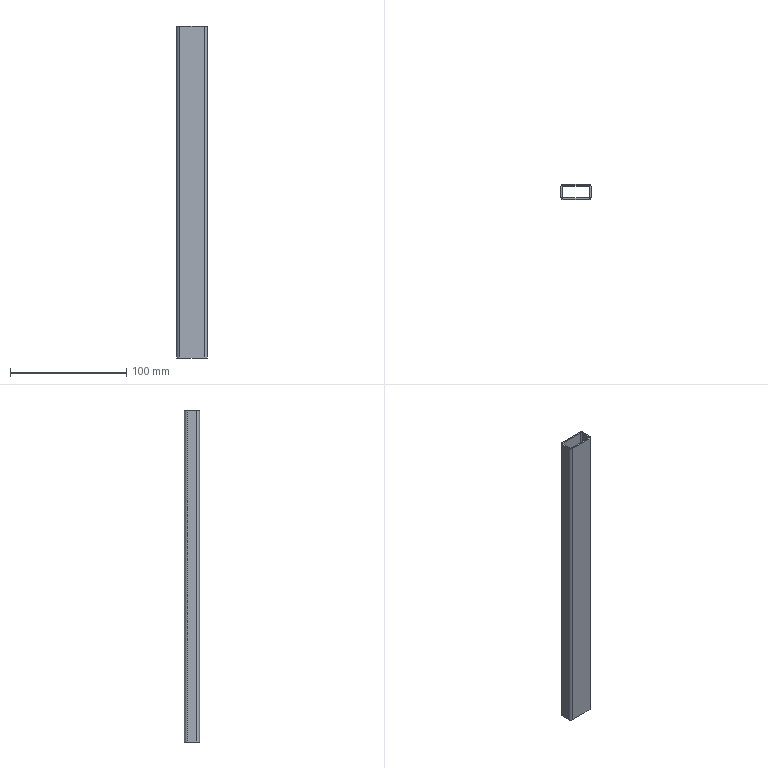Part | STEP file | Q7C0515 | 1 solid | 18 faces | box 26 x 13 x 285 mm | volume 23919 mm3 | plane 10 | cylinder 8 | commonest cylinder face diameters 2.6 x4 5 x4
STEP:
#1=CARTESIAN_POINT('',(0.,0.,0.));
#2=DIRECTION('',(0.,0.,1.));
#3=DIRECTION('',(1.,0.,0.));
#4=AXIS2_PLACEMENT_3D('',#1,#2,#3);
#5=CARTESIAN_POINT('',(13.,4.,142.5));
#6=VERTEX_POINT('',#5);
#7=CARTESIAN_POINT('',(10.5,6.5,142.5));
#8=VERTEX_POINT('',#7);
#9=CARTESIAN_POINT('',(10.5,4.,142.5));
#10=DIRECTION('',(0.,0.,1.));
#11=DIRECTION('',(-1.,0.,0.));
#12=AXIS2_PLACEMENT_3D('',#9,#10,#11);
#13=CIRCLE('',#12,2.5);
#14=CARTESIAN_POINT('',(10.5,4.,142.5));
#15=DIRECTION('',(0.,0.,-1.));
#16=DIRECTION('',(-1.,0.,0.));
#17=AXIS2_PLACEMENT_3D('',#14,#15,#16);
#18=PLANE('',#17);
#19=CARTESIAN_POINT('',(2.5,0.));
#20=CARTESIAN_POINT('',(2.5,-4.33));
#21=CARTESIAN_POINT('',(-1.25,-2.165));
#22=CARTESIAN_POINT('',(-5.,0.));
#23=CARTESIAN_POINT('',(-1.25,2.165));
#24=CARTESIAN_POINT('',(2.5,4.33));
#25=CARTESIAN_POINT('',(2.5,0.));
#26=(BOUNDED_CURVE()B_SPLINE_CURVE(2,(#19,#20,#21,#22,#23,#24,#25),.UNSPECIFIED.,.T.,.F.)B_SPLINE_CURVE_WITH_KNOTS((1,2,2,2,2,1),(-2.094,0.,2.094,4.189,6.283,8.378),.UNSPECIFIED.)CURVE()GEOMETRIC_REPRESENTATION_ITEM()RATIONAL_B_SPLINE_CURVE((1.,0.5,1.,0.5,1.,0.5,1.))REPRESENTATION_ITEM(''));
#27=(GEOMETRIC_REPRESENTATION_CONTEXT(2)PARAMETRIC_REPRESENTATION_CONTEXT()REPRESENTATION_CONTEXT('',''));
#28=DEFINITIONAL_REPRESENTATION('',(#26),#27);
#29=PCURVE('',#18,#28);
#30=CARTESIAN_POINT('',(10.5,4.,142.5));
#31=DIRECTION('',(0.,0.,-1.));
#32=DIRECTION('',(-1.,0.,0.));
#33=AXIS2_PLACEMENT_3D('',#30,#31,#32);
#34=CYLINDRICAL_SURFACE('',#33,2.5);
#35=CARTESIAN_POINT('',(6.283,0.));
#36=DIRECTION('',(-1.,0.));
#37=VECTOR('',#36,1.);
#38=LINE('',#35,#37);
#39=(GEOMETRIC_REPRESENTATION_CONTEXT(2)PARAMETRIC_REPRESENTATION_CONTEXT()REPRESENTATION_CONTEXT('',''));
#40=DEFINITIONAL_REPRESENTATION('',(#38),#39);
#41=PCURVE('',#34,#40);
#42=SURFACE_CURVE('',#13,(#29,#41),.PCURVE_S1.);
#43=EDGE_CURVE('',#6,#8,#42,.T.);
#44=ORIENTED_EDGE('',*,*,#43,.T.);
#45=CARTESIAN_POINT('',(-10.5,6.5,142.5));
#46=VERTEX_POINT('',#45);
#47=CARTESIAN_POINT('',(-10.5,6.5,142.5));
#48=DIRECTION('',(-1.,0.,0.));
#49=VECTOR('',#48,1.);
#50=LINE('',#47,#49);
#51=CARTESIAN_POINT('',(21.,2.5));
#52=DIRECTION('',(1.,0.));
#53=VECTOR('',#52,1.);
#54=LINE('',#51,#53);
#55=(GEOMETRIC_REPRESENTATION_CONTEXT(2)PARAMETRIC_REPRESENTATION_CONTEXT()REPRESENTATION_CONTEXT('',''));
#56=DEFINITIONAL_REPRESENTATION('',(#54),#55);
#57=PCURVE('',#18,#56);
#58=CARTESIAN_POINT('',(-10.5,6.5,142.5));
#59=DIRECTION('',(0.,-1.,0.));
#60=DIRECTION('',(1.,0.,0.));
#61=AXIS2_PLACEMENT_3D('',#58,#59,#60);
#62=PLANE('',#61);
#63=CARTESIAN_POINT('',(0.,0.));
#64=DIRECTION('',(-1.,0.));
#65=VECTOR('',#64,1.);
#66=LINE('',#63,#65);
#67=(GEOMETRIC_REPRESENTATION_CONTEXT(2)PARAMETRIC_REPRESENTATION_CONTEXT()REPRESENTATION_CONTEXT('',''));
#68=DEFINITIONAL_REPRESENTATION('',(#66),#67);
#69=PCURVE('',#62,#68);
#70=SURFACE_CURVE('',#50,(#57,#69),.PCURVE_S1.);
#71=EDGE_CURVE('',#8,#46,#70,.T.);
#72=ORIENTED_EDGE('',*,*,#71,.T.);
#73=CARTESIAN_POINT('',(-13.,4.,142.5));
#74=VERTEX_POINT('',#73);
#75=CARTESIAN_POINT('',(-10.5,4.,142.5));
#76=DIRECTION('',(0.,0.,1.));
#77=DIRECTION('',(1.,0.,0.));
#78=AXIS2_PLACEMENT_3D('',#75,#76,#77);
#79=CIRCLE('',#78,2.5);
#80=CARTESIAN_POINT('',(18.5,0.));
#81=CARTESIAN_POINT('',(18.5,4.33));
#82=CARTESIAN_POINT('',(22.25,2.165));
#83=CARTESIAN_POINT('',(26.,0.));
#84=CARTESIAN_POINT('',(22.25,-2.165));
#85=CARTESIAN_POINT('',(18.5,-4.33));
#86=CARTESIAN_POINT('',(18.5,0.));
#87=(BOUNDED_CURVE()B_SPLINE_CURVE(2,(#80,#81,#82,#83,#84,#85,#86),.UNSPECIFIED.,.T.,.F.)B_SPLINE_CURVE_WITH_KNOTS((1,2,2,2,2,1),(-2.094,0.,2.094,4.189,6.283,8.378),.UNSPECIFIED.)CURVE()GEOMETRIC_REPRESENTATION_ITEM()RATIONAL_B_SPLINE_CURVE((1.,0.5,1.,0.5,1.,0.5,1.))REPRESENTATION_ITEM(''));
#88=(GEOMETRIC_REPRESENTATION_CONTEXT(2)PARAMETRIC_REPRESENTATION_CONTEXT()REPRESENTATION_CONTEXT('',''));
#89=DEFINITIONAL_REPRESENTATION('',(#87),#88);
#90=PCURVE('',#18,#89);
#91=CARTESIAN_POINT('',(-10.5,4.,142.5));
#92=DIRECTION('',(0.,0.,-1.));
#93=DIRECTION('',(-1.,0.,0.));
#94=AXIS2_PLACEMENT_3D('',#91,#92,#93);
#95=CYLINDRICAL_SURFACE('',#94,2.5);
#96=CARTESIAN_POINT('',(3.142,0.));
#97=DIRECTION('',(-1.,0.));
#98=VECTOR('',#97,1.);
#99=LINE('',#96,#98);
#100=(GEOMETRIC_REPRESENTATION_CONTEXT(2)PARAMETRIC_REPRESENTATION_CONTEXT()REPRESENTATION_CONTEXT('',''));
#101=DEFINITIONAL_REPRESENTATION('',(#99),#100);
#102=PCURVE('',#95,#101);
#103=SURFACE_CURVE('',#79,(#90,#102),.PCURVE_S1.);
#104=EDGE_CURVE('',#46,#74,#103,.T.);
#105=ORIENTED_EDGE('',*,*,#104,.T.);
#106=CARTESIAN_POINT('',(-13.,-4.,142.5));
#107=VERTEX_POINT('',#106);
#108=CARTESIAN_POINT('',(-13.,4.,142.5));
#109=DIRECTION('',(0.,-1.,0.));
#110=VECTOR('',#109,1.);
#111=LINE('',#108,#110);
#112=CARTESIAN_POINT('',(23.5,0.));
#113=DIRECTION('',(0.,-1.));
#114=VECTOR('',#113,1.);
#115=LINE('',#112,#114);
#116=(GEOMETRIC_REPRESENTATION_CONTEXT(2)PARAMETRIC_REPRESENTATION_CONTEXT()REPRESENTATION_CONTEXT('',''));
#117=DEFINITIONAL_REPRESENTATION('',(#115),#116);
#118=PCURVE('',#18,#117);
#119=CARTESIAN_POINT('',(-13.,4.,142.5));
#120=DIRECTION('',(1.,0.,0.));
#121=DIRECTION('',(0.,0.,-1.));
#122=AXIS2_PLACEMENT_3D('',#119,#120,#121);
#123=PLANE('',#122);
#124=CARTESIAN_POINT('',(0.,0.));
#125=DIRECTION('',(0.,-1.));
#126=VECTOR('',#125,1.);
#127=LINE('',#124,#126);
#128=(GEOMETRIC_REPRESENTATION_CONTEXT(2)PARAMETRIC_REPRESENTATION_CONTEXT()REPRESENTATION_CONTEXT('',''));
#129=DEFINITIONAL_REPRESENTATION('',(#127),#128);
#130=PCURVE('',#123,#129);
#131=SURFACE_CURVE('',#111,(#118,#130),.PCURVE_S1.);
#132=EDGE_CURVE('',#74,#107,#131,.T.);
#133=ORIENTED_EDGE('',*,*,#132,.T.);
#134=CARTESIAN_POINT('',(-10.5,-6.5,142.5));
#135=VERTEX_POINT('',#134);
#136=CARTESIAN_POINT('',(-10.5,-4.,142.5));
#137=DIRECTION('',(0.,0.,1.));
#138=DIRECTION('',(1.,0.,0.));
#139=AXIS2_PLACEMENT_3D('',#136,#137,#138);
#140=CIRCLE('',#139,2.5);
#141=CARTESIAN_POINT('',(18.5,-8.));
#142=CARTESIAN_POINT('',(18.5,-3.67));
#143=CARTESIAN_POINT('',(22.25,-5.835));
#144=CARTESIAN_POINT('',(26.,-8.));
#145=CARTESIAN_POINT('',(22.25,-10.165));
#146=CARTESIAN_POINT('',(18.5,-12.33));
#147=CARTESIAN_POINT('',(18.5,-8.));
#148=(BOUNDED_CURVE()B_SPLINE_CURVE(2,(#141,#142,#143,#144,#145,#146,#147),.UNSPECIFIED.,.T.,.F.)B_SPLINE_CURVE_WITH_KNOTS((1,2,2,2,2,1),(-2.094,0.,2.094,4.189,6.283,8.378),.UNSPECIFIED.)CURVE()GEOMETRIC_REPRESENTATION_ITEM()RATIONAL_B_SPLINE_CURVE((1.,0.5,1.,0.5,1.,0.5,1.))REPRESENTATION_ITEM(''));
#149=(GEOMETRIC_REPRESENTATION_CONTEXT(2)PARAMETRIC_REPRESENTATION_CONTEXT()REPRESENTATION_CONTEXT('',''));
#150=DEFINITIONAL_REPRESENTATION('',(#148),#149);
#151=PCURVE('',#18,#150);
#152=CARTESIAN_POINT('',(-10.5,-4.,142.5));
#153=DIRECTION('',(0.,0.,-1.));
#154=DIRECTION('',(-1.,0.,0.));
#155=AXIS2_PLACEMENT_3D('',#152,#153,#154);
#156=CYLINDRICAL_SURFACE('',#155,2.5);
#157=CARTESIAN_POINT('',(9.425,0.));
#158=DIRECTION('',(-1.,0.));
#159=VECTOR('',#158,1.);
#160=LINE('',#157,#159);
#161=(GEOMETRIC_REPRESENTATION_CONTEXT(2)PARAMETRIC_REPRESENTATION_CONTEXT()REPRESENTATION_CONTEXT('',''));
#162=DEFINITIONAL_REPRESENTATION('',(#160),#161);
#163=PCURVE('',#156,#162);
#164=SURFACE_CURVE('',#140,(#151,#163),.PCURVE_S1.);
#165=EDGE_CURVE('',#107,#135,#164,.T.);
#166=ORIENTED_EDGE('',*,*,#165,.T.);
#167=CARTESIAN_POINT('',(10.5,-6.5,142.5));
#168=VERTEX_POINT('',#167);
#169=CARTESIAN_POINT('',(-10.5,-6.5,142.5));
#170=DIRECTION('',(1.,0.,0.));
#171=VECTOR('',#170,1.);
#172=LINE('',#169,#171);
#173=CARTESIAN_POINT('',(21.,-10.5));
#174=DIRECTION('',(-1.,0.));
#175=VECTOR('',#174,1.);
#176=LINE('',#173,#175);
#177=(GEOMETRIC_REPRESENTATION_CONTEXT(2)PARAMETRIC_REPRESENTATION_CONTEXT()REPRESENTATION_CONTEXT('',''));
#178=DEFINITIONAL_REPRESENTATION('',(#176),#177);
#179=PCURVE('',#18,#178);
#180=CARTESIAN_POINT('',(-10.5,-6.5,142.5));
#181=DIRECTION('',(0.,1.,0.));
#182=DIRECTION('',(0.,0.,1.));
#183=AXIS2_PLACEMENT_3D('',#180,#181,#182);
#184=PLANE('',#183);
#185=CARTESIAN_POINT('',(0.,0.));
#186=DIRECTION('',(0.,1.));
#187=VECTOR('',#186,1.);
#188=LINE('',#185,#187);
#189=(GEOMETRIC_REPRESENTATION_CONTEXT(2)PARAMETRIC_REPRESENTATION_CONTEXT()REPRESENTATION_CONTEXT('',''));
#190=DEFINITIONAL_REPRESENTATION('',(#188),#189);
#191=PCURVE('',#184,#190);
#192=SURFACE_CURVE('',#172,(#179,#191),.PCURVE_S1.);
#193=EDGE_CURVE('',#135,#168,#192,.T.);
#194=ORIENTED_EDGE('',*,*,#193,.T.);
#195=CARTESIAN_POINT('',(13.,-4.,142.5));
#196=VERTEX_POINT('',#195);
#197=CARTESIAN_POINT('',(10.5,-4.,142.5));
#198=DIRECTION('',(0.,0.,1.));
#199=DIRECTION('',(-1.,0.,0.));
#200=AXIS2_PLACEMENT_3D('',#197,#198,#199);
#201=CIRCLE('',#200,2.5);
#202=CARTESIAN_POINT('',(2.5,-8.));
#203=CARTESIAN_POINT('',(2.5,-12.33));
#204=CARTESIAN_POINT('',(-1.25,-10.165));
#205=CARTESIAN_POINT('',(-5.,-8.));
#206=CARTESIAN_POINT('',(-1.25,-5.835));
#207=CARTESIAN_POINT('',(2.5,-3.67));
#208=CARTESIAN_POINT('',(2.5,-8.));
#209=(BOUNDED_CURVE()B_SPLINE_CURVE(2,(#202,#203,#204,#205,#206,#207,#208),.UNSPECIFIED.,.T.,.F.)B_SPLINE_CURVE_WITH_KNOTS((1,2,2,2,2,1),(-2.094,0.,2.094,4.189,6.283,8.378),.UNSPECIFIED.)CURVE()GEOMETRIC_REPRESENTATION_ITEM()RATIONAL_B_SPLINE_CURVE((1.,0.5,1.,0.5,1.,0.5,1.))REPRESENTATION_ITEM(''));
#210=(GEOMETRIC_REPRESENTATION_CONTEXT(2)PARAMETRIC_REPRESENTATION_CONTEXT()REPRESENTATION_CONTEXT('',''));
#211=DEFINITIONAL_REPRESENTATION('',(#209),#210);
#212=PCURVE('',#18,#211);
#213=CARTESIAN_POINT('',(10.5,-4.,142.5));
#214=DIRECTION('',(0.,0.,-1.));
#215=DIRECTION('',(-1.,0.,0.));
#216=AXIS2_PLACEMENT_3D('',#213,#214,#215);
#217=CYLINDRICAL_SURFACE('',#216,2.5);
#218=CARTESIAN_POINT('',(6.283,0.));
#219=DIRECTION('',(-1.,0.));
#220=VECTOR('',#219,1.);
#221=LINE('',#218,#220);
#222=(GEOMETRIC_REPRESENTATION_CONTEXT(2)PARAMETRIC_REPRESENTATION_CONTEXT()REPRESENTATION_CONTEXT('',''));
#223=DEFINITIONAL_REPRESENTATION('',(#221),#222);
#224=PCURVE('',#217,#223);
#225=SURFACE_CURVE('',#201,(#212,#224),.PCURVE_S1.);
#226=EDGE_CURVE('',#168,#196,#225,.T.);
#227=ORIENTED_EDGE('',*,*,#226,.T.);
#228=CARTESIAN_POINT('',(13.,4.,142.5));
#229=DIRECTION('',(0.,1.,0.));
#230=VECTOR('',#229,1.);
#231=LINE('',#228,#230);
#232=CARTESIAN_POINT('',(-2.5,0.));
#233=DIRECTION('',(0.,1.));
#234=VECTOR('',#233,1.);
#235=LINE('',#232,#234);
#236=(GEOMETRIC_REPRESENTATION_CONTEXT(2)PARAMETRIC_REPRESENTATION_CONTEXT()REPRESENTATION_CONTEXT('',''));
#237=DEFINITIONAL_REPRESENTATION('',(#235),#236);
#238=PCURVE('',#18,#237);
#239=CARTESIAN_POINT('',(13.,4.,142.5));
#240=DIRECTION('',(-1.,0.,0.));
#241=DIRECTION('',(0.,-1.,0.));
#242=AXIS2_PLACEMENT_3D('',#239,#240,#241);
#243=PLANE('',#242);
#244=CARTESIAN_POINT('',(0.,0.));
#245=DIRECTION('',(-1.,0.));
#246=VECTOR('',#245,1.);
#247=LINE('',#244,#246);
#248=(GEOMETRIC_REPRESENTATION_CONTEXT(2)PARAMETRIC_REPRESENTATION_CONTEXT()REPRESENTATION_CONTEXT('',''));
#249=DEFINITIONAL_REPRESENTATION('',(#247),#248);
#250=PCURVE('',#243,#249);
#251=SURFACE_CURVE('',#231,(#238,#250),.PCURVE_S1.);
#252=EDGE_CURVE('',#196,#6,#251,.T.);
#253=ORIENTED_EDGE('',*,*,#252,.T.);
#254=EDGE_LOOP('',(#44,#72,#105,#133,#166,#194,#227,#253));
#255=FACE_BOUND('',#254,.T.);
#256=CARTESIAN_POINT('',(-10.5,5.3,142.5));
#257=VERTEX_POINT('',#256);
#258=CARTESIAN_POINT('',(-11.8,4.,142.5));
#259=VERTEX_POINT('',#258);
#260=CARTESIAN_POINT('',(-10.5,4.,142.5));
#261=DIRECTION('',(0.,0.,1.));
#262=DIRECTION('',(1.,0.,0.));
#263=AXIS2_PLACEMENT_3D('',#260,#261,#262);
#264=CIRCLE('',#263,1.3);
#265=CARTESIAN_POINT('',(19.7,0.));
#266=CARTESIAN_POINT('',(19.7,2.252));
#267=CARTESIAN_POINT('',(21.65,1.126));
#268=CARTESIAN_POINT('',(23.6,0.));
#269=CARTESIAN_POINT('',(21.65,-1.126));
#270=CARTESIAN_POINT('',(19.7,-2.252));
#271=CARTESIAN_POINT('',(19.7,0.));
#272=(BOUNDED_CURVE()B_SPLINE_CURVE(2,(#265,#266,#267,#268,#269,#270,#271),.UNSPECIFIED.,.T.,.F.)B_SPLINE_CURVE_WITH_KNOTS((1,2,2,2,2,1),(-2.094,0.,2.094,4.189,6.283,8.378),.UNSPECIFIED.)CURVE()GEOMETRIC_REPRESENTATION_ITEM()RATIONAL_B_SPLINE_CURVE((1.,0.5,1.,0.5,1.,0.5,1.))REPRESENTATION_ITEM(''));
#273=(GEOMETRIC_REPRESENTATION_CONTEXT(2)PARAMETRIC_REPRESENTATION_CONTEXT()REPRESENTATION_CONTEXT('',''));
#274=DEFINITIONAL_REPRESENTATION('',(#272),#273);
#275=PCURVE('',#18,#274);
#276=CARTESIAN_POINT('',(-10.5,4.,142.5));
#277=DIRECTION('',(0.,0.,-1.));
#278=DIRECTION('',(-1.,0.,0.));
#279=AXIS2_PLACEMENT_3D('',#276,#277,#278);
#280=CYLINDRICAL_SURFACE('',#279,1.3);
#281=CARTESIAN_POINT('',(3.142,0.));
#282=DIRECTION('',(-1.,0.));
#283=VECTOR('',#282,1.);
#284=LINE('',#281,#283);
#285=(GEOMETRIC_REPRESENTATION_CONTEXT(2)PARAMETRIC_REPRESENTATION_CONTEXT()REPRESENTATION_CONTEXT('',''));
#286=DEFINITIONAL_REPRESENTATION('',(#284),#285);
#287=PCURVE('',#280,#286);
#288=SURFACE_CURVE('',#264,(#275,#287),.PCURVE_S1.);
#289=EDGE_CURVE('',#257,#259,#288,.T.);
#290=ORIENTED_EDGE('',*,*,#289,.F.);
#291=CARTESIAN_POINT('',(10.5,5.3,142.5));
#292=VERTEX_POINT('',#291);
#293=CARTESIAN_POINT('',(-10.5,5.3,142.5));
#294=DIRECTION('',(-1.,0.,0.));
#295=VECTOR('',#294,1.);
#296=LINE('',#293,#295);
#297=CARTESIAN_POINT('',(21.,1.3));
#298=DIRECTION('',(1.,0.));
#299=VECTOR('',#298,1.);
#300=LINE('',#297,#299);
#301=(GEOMETRIC_REPRESENTATION_CONTEXT(2)PARAMETRIC_REPRESENTATION_CONTEXT()REPRESENTATION_CONTEXT('',''));
#302=DEFINITIONAL_REPRESENTATION('',(#300),#301);
#303=PCURVE('',#18,#302);
#304=CARTESIAN_POINT('',(-10.5,5.3,142.5));
#305=DIRECTION('',(0.,-1.,0.));
#306=DIRECTION('',(0.,0.,-1.));
#307=AXIS2_PLACEMENT_3D('',#304,#305,#306);
#308=PLANE('',#307);
#309=CARTESIAN_POINT('',(0.,0.));
#310=DIRECTION('',(0.,-1.));
#311=VECTOR('',#310,1.);
#312=LINE('',#309,#311);
#313=(GEOMETRIC_REPRESENTATION_CONTEXT(2)PARAMETRIC_REPRESENTATION_CONTEXT()REPRESENTATION_CONTEXT('',''));
#314=DEFINITIONAL_REPRESENTATION('',(#312),#313);
#315=PCURVE('',#308,#314);
#316=SURFACE_CURVE('',#296,(#303,#315),.PCURVE_S1.);
#317=EDGE_CURVE('',#292,#257,#316,.T.);
#318=ORIENTED_EDGE('',*,*,#317,.F.);
#319=CARTESIAN_POINT('',(11.8,4.,142.5));
#320=VERTEX_POINT('',#319);
#321=CARTESIAN_POINT('',(10.5,4.,142.5));
#322=DIRECTION('',(0.,0.,1.));
#323=DIRECTION('',(-1.,0.,0.));
#324=AXIS2_PLACEMENT_3D('',#321,#322,#323);
#325=CIRCLE('',#324,1.3);
#326=CARTESIAN_POINT('',(1.3,0.));
#327=CARTESIAN_POINT('',(1.3,-2.252));
#328=CARTESIAN_POINT('',(-0.65,-1.126));
#329=CARTESIAN_POINT('',(-2.6,0.));
#330=CARTESIAN_POINT('',(-0.65,1.126));
#331=CARTESIAN_POINT('',(1.3,2.252));
#332=CARTESIAN_POINT('',(1.3,0.));
#333=(BOUNDED_CURVE()B_SPLINE_CURVE(2,(#326,#327,#328,#329,#330,#331,#332),.UNSPECIFIED.,.T.,.F.)B_SPLINE_CURVE_WITH_KNOTS((1,2,2,2,2,1),(-2.094,0.,2.094,4.189,6.283,8.378),.UNSPECIFIED.)CURVE()GEOMETRIC_REPRESENTATION_ITEM()RATIONAL_B_SPLINE_CURVE((1.,0.5,1.,0.5,1.,0.5,1.))REPRESENTATION_ITEM(''));
#334=(GEOMETRIC_REPRESENTATION_CONTEXT(2)PARAMETRIC_REPRESENTATION_CONTEXT()REPRESENTATION_CONTEXT('',''));
#335=DEFINITIONAL_REPRESENTATION('',(#333),#334);
#336=PCURVE('',#18,#335);
#337=CARTESIAN_POINT('',(10.5,4.,142.5));
#338=DIRECTION('',(0.,0.,-1.));
#339=DIRECTION('',(-1.,0.,0.));
#340=AXIS2_PLACEMENT_3D('',#337,#338,#339);
#341=CYLINDRICAL_SURFACE('',#340,1.3);
#342=CARTESIAN_POINT('',(6.283,0.));
#343=DIRECTION('',(-1.,0.));
#344=VECTOR('',#343,1.);
#345=LINE('',#342,#344);
#346=(GEOMETRIC_REPRESENTATION_CONTEXT(2)PARAMETRIC_REPRESENTATION_CONTEXT()REPRESENTATION_CONTEXT('',''));
#347=DEFINITIONAL_REPRESENTATION('',(#345),#346);
#348=PCURVE('',#341,#347);
#349=SURFACE_CURVE('',#325,(#336,#348),.PCURVE_S1.);
#350=EDGE_CURVE('',#320,#292,#349,.T.);
#351=ORIENTED_EDGE('',*,*,#350,.F.);
#352=CARTESIAN_POINT('',(11.8,-4.,142.5));
#353=VERTEX_POINT('',#352);
#354=CARTESIAN_POINT('',(11.8,4.,142.5));
#355=DIRECTION('',(0.,1.,0.));
#356=VECTOR('',#355,1.);
#357=LINE('',#354,#356);
#358=CARTESIAN_POINT('',(-1.3,0.));
#359=DIRECTION('',(0.,1.));
#360=VECTOR('',#359,1.);
#361=LINE('',#358,#360);
#362=(GEOMETRIC_REPRESENTATION_CONTEXT(2)PARAMETRIC_REPRESENTATION_CONTEXT()REPRESENTATION_CONTEXT('',''));
#363=DEFINITIONAL_REPRESENTATION('',(#361),#362);
#364=PCURVE('',#18,#363);
#365=CARTESIAN_POINT('',(11.8,4.,142.5));
#366=DIRECTION('',(-1.,0.,0.));
#367=DIRECTION('',(0.,-1.,0.));
#368=AXIS2_PLACEMENT_3D('',#365,#366,#367);
#369=PLANE('',#368);
#370=CARTESIAN_POINT('',(0.,0.));
#371=DIRECTION('',(-1.,0.));
#372=VECTOR('',#371,1.);
#373=LINE('',#370,#372);
#374=(GEOMETRIC_REPRESENTATION_CONTEXT(2)PARAMETRIC_REPRESENTATION_CONTEXT()REPRESENTATION_CONTEXT('',''));
#375=DEFINITIONAL_REPRESENTATION('',(#373),#374);
#376=PCURVE('',#369,#375);
#377=SURFACE_CURVE('',#357,(#364,#376),.PCURVE_S1.);
#378=EDGE_CURVE('',#353,#320,#377,.T.);
#379=ORIENTED_EDGE('',*,*,#378,.F.);
#380=CARTESIAN_POINT('',(10.5,-5.3,142.5));
#381=VERTEX_POINT('',#380);
#382=CARTESIAN_POINT('',(10.5,-4.,142.5));
#383=DIRECTION('',(0.,0.,1.));
#384=DIRECTION('',(-1.,0.,0.));
#385=AXIS2_PLACEMENT_3D('',#382,#383,#384);
#386=CIRCLE('',#385,1.3);
#387=CARTESIAN_POINT('',(1.3,-8.));
#388=CARTESIAN_POINT('',(1.3,-10.252));
#389=CARTESIAN_POINT('',(-0.65,-9.126));
#390=CARTESIAN_POINT('',(-2.6,-8.));
#391=CARTESIAN_POINT('',(-0.65,-6.874));
#392=CARTESIAN_POINT('',(1.3,-5.748));
#393=CARTESIAN_POINT('',(1.3,-8.));
#394=(BOUNDED_CURVE()B_SPLINE_CURVE(2,(#387,#388,#389,#390,#391,#392,#393),.UNSPECIFIED.,.T.,.F.)B_SPLINE_CURVE_WITH_KNOTS((1,2,2,2,2,1),(-2.094,0.,2.094,4.189,6.283,8.378),.UNSPECIFIED.)CURVE()GEOMETRIC_REPRESENTATION_ITEM()RATIONAL_B_SPLINE_CURVE((1.,0.5,1.,0.5,1.,0.5,1.))REPRESENTATION_ITEM(''));
#395=(GEOMETRIC_REPRESENTATION_CONTEXT(2)PARAMETRIC_REPRESENTATION_CONTEXT()REPRESENTATION_CONTEXT('',''));
#396=DEFINITIONAL_REPRESENTATION('',(#394),#395);
#397=PCURVE('',#18,#396);
#398=CARTESIAN_POINT('',(10.5,-4.,142.5));
#399=DIRECTION('',(0.,0.,-1.));
#400=DIRECTION('',(-1.,0.,0.));
#401=AXIS2_PLACEMENT_3D('',#398,#399,#400);
#402=CYLINDRICAL_SURFACE('',#401,1.3);
#403=CARTESIAN_POINT('',(6.283,0.));
#404=DIRECTION('',(-1.,0.));
#405=VECTOR('',#404,1.);
#406=LINE('',#403,#405);
#407=(GEOMETRIC_REPRESENTATION_CONTEXT(2)PARAMETRIC_REPRESENTATION_CONTEXT()REPRESENTATION_CONTEXT('',''));
#408=DEFINITIONAL_REPRESENTATION('',(#406),#407);
#409=PCURVE('',#402,#408);
#410=SURFACE_CURVE('',#386,(#397,#409),.PCURVE_S1.);
#411=EDGE_CURVE('',#381,#353,#410,.T.);
#412=ORIENTED_EDGE('',*,*,#411,.F.);
#413=CARTESIAN_POINT('',(-10.5,-5.3,142.5));
#414=VERTEX_POINT('',#413);
#415=CARTESIAN_POINT('',(-10.5,-5.3,142.5));
#416=DIRECTION('',(1.,0.,0.));
#417=VECTOR('',#416,1.);
#418=LINE('',#415,#417);
#419=CARTESIAN_POINT('',(21.,-9.3));
#420=DIRECTION('',(-1.,0.));
#421=VECTOR('',#420,1.);
#422=LINE('',#419,#421);
#423=(GEOMETRIC_REPRESENTATION_CONTEXT(2)PARAMETRIC_REPRESENTATION_CONTEXT()REPRESENTATION_CONTEXT('',''));
#424=DEFINITIONAL_REPRESENTATION('',(#422),#423);
#425=PCURVE('',#18,#424);
#426=CARTESIAN_POINT('',(-10.5,-5.3,142.5));
#427=DIRECTION('',(0.,1.,0.));
#428=DIRECTION('',(0.,0.,1.));
#429=AXIS2_PLACEMENT_3D('',#426,#427,#428);
#430=PLANE('',#429);
#431=CARTESIAN_POINT('',(0.,0.));
#432=DIRECTION('',(0.,1.));
#433=VECTOR('',#432,1.);
#434=LINE('',#431,#433);
#435=(GEOMETRIC_REPRESENTATION_CONTEXT(2)PARAMETRIC_REPRESENTATION_CONTEXT()REPRESENTATION_CONTEXT('',''));
#436=DEFINITIONAL_REPRESENTATION('',(#434),#435);
#437=PCURVE('',#430,#436);
#438=SURFACE_CURVE('',#418,(#425,#437),.PCURVE_S1.);
#439=EDGE_CURVE('',#414,#381,#438,.T.);
#440=ORIENTED_EDGE('',*,*,#439,.F.);
#441=CARTESIAN_POINT('',(-11.8,-4.,142.5));
#442=VERTEX_POINT('',#441);
#443=CARTESIAN_POINT('',(-10.5,-4.,142.5));
#444=DIRECTION('',(0.,0.,1.));
#445=DIRECTION('',(1.,0.,0.));
#446=AXIS2_PLACEMENT_3D('',#443,#444,#445);
#447=CIRCLE('',#446,1.3);
#448=CARTESIAN_POINT('',(19.7,-8.));
#449=CARTESIAN_POINT('',(19.7,-5.748));
#450=CARTESIAN_POINT('',(21.65,-6.874));
#451=CARTESIAN_POINT('',(23.6,-8.));
#452=CARTESIAN_POINT('',(21.65,-9.126));
#453=CARTESIAN_POINT('',(19.7,-10.252));
#454=CARTESIAN_POINT('',(19.7,-8.));
#455=(BOUNDED_CURVE()B_SPLINE_CURVE(2,(#448,#449,#450,#451,#452,#453,#454),.UNSPECIFIED.,.T.,.F.)B_SPLINE_CURVE_WITH_KNOTS((1,2,2,2,2,1),(-2.094,0.,2.094,4.189,6.283,8.378),.UNSPECIFIED.)CURVE()GEOMETRIC_REPRESENTATION_ITEM()RATIONAL_B_SPLINE_CURVE((1.,0.5,1.,0.5,1.,0.5,1.))REPRESENTATION_ITEM(''));
#456=(GEOMETRIC_REPRESENTATION_CONTEXT(2)PARAMETRIC_REPRESENTATION_CONTEXT()REPRESENTATION_CONTEXT('',''));
#457=DEFINITIONAL_REPRESENTATION('',(#455),#456);
#458=PCURVE('',#18,#457);
#459=CARTESIAN_POINT('',(-10.5,-4.,142.5));
#460=DIRECTION('',(0.,0.,-1.));
#461=DIRECTION('',(-1.,0.,0.));
#462=AXIS2_PLACEMENT_3D('',#459,#460,#461);
#463=CYLINDRICAL_SURFACE('',#462,1.3);
#464=CARTESIAN_POINT('',(9.425,0.));
#465=DIRECTION('',(-1.,0.));
#466=VECTOR('',#465,1.);
#467=LINE('',#464,#466);
#468=(GEOMETRIC_REPRESENTATION_CONTEXT(2)PARAMETRIC_REPRESENTATION_CONTEXT()REPRESENTATION_CONTEXT('',''));
#469=DEFINITIONAL_REPRESENTATION('',(#467),#468);
#470=PCURVE('',#463,#469);
#471=SURFACE_CURVE('',#447,(#458,#470),.PCURVE_S1.);
#472=EDGE_CURVE('',#442,#414,#471,.T.);
#473=ORIENTED_EDGE('',*,*,#472,.F.);
#474=CARTESIAN_POINT('',(-11.8,4.,142.5));
#475=DIRECTION('',(0.,-1.,0.));
#476=VECTOR('',#475,1.);
#477=LINE('',#474,#476);
#478=CARTESIAN_POINT('',(22.3,0.));
#479=DIRECTION('',(0.,-1.));
#480=VECTOR('',#479,1.);
#481=LINE('',#478,#480);
#482=(GEOMETRIC_REPRESENTATION_CONTEXT(2)PARAMETRIC_REPRESENTATION_CONTEXT()REPRESENTATION_CONTEXT('',''));
#483=DEFINITIONAL_REPRESENTATION('',(#481),#482);
#484=PCURVE('',#18,#483);
#485=CARTESIAN_POINT('',(-11.8,4.,142.5));
#486=DIRECTION('',(1.,0.,0.));
#487=DIRECTION('',(0.,1.,0.));
#488=AXIS2_PLACEMENT_3D('',#485,#486,#487);
#489=PLANE('',#488);
#490=CARTESIAN_POINT('',(0.,0.));
#491=DIRECTION('',(-1.,0.));
#492=VECTOR('',#491,1.);
#493=LINE('',#490,#492);
#494=(GEOMETRIC_REPRESENTATION_CONTEXT(2)PARAMETRIC_REPRESENTATION_CONTEXT()REPRESENTATION_CONTEXT('',''));
#495=DEFINITIONAL_REPRESENTATION('',(#493),#494);
#496=PCURVE('',#489,#495);
#497=SURFACE_CURVE('',#477,(#484,#496),.PCURVE_S1.);
#498=EDGE_CURVE('',#259,#442,#497,.T.);
#499=ORIENTED_EDGE('',*,*,#498,.F.);
#500=EDGE_LOOP('',(#290,#318,#351,#379,#412,#440,#473,#499));
#501=FACE_BOUND('',#500,.T.);
#502=ADVANCED_FACE('',(#255,#501),#18,.F.);
#503=CARTESIAN_POINT('',(13.,4.,-142.5));
#504=VERTEX_POINT('',#503);
#505=CARTESIAN_POINT('',(10.5,6.5,-142.5));
#506=VERTEX_POINT('',#505);
#507=CARTESIAN_POINT('',(10.5,4.,-142.5));
#508=DIRECTION('',(0.,0.,1.));
#509=DIRECTION('',(-1.,0.,0.));
#510=AXIS2_PLACEMENT_3D('',#507,#508,#509);
#511=CIRCLE('',#510,2.5);
#512=CARTESIAN_POINT('',(10.5,4.,-142.5));
#513=DIRECTION('',(0.,0.,-1.));
#514=DIRECTION('',(-1.,0.,0.));
#515=AXIS2_PLACEMENT_3D('',#512,#513,#514);
#516=PLANE('',#515);
#517=CARTESIAN_POINT('',(2.5,0.));
#518=CARTESIAN_POINT('',(2.5,-4.33));
#519=CARTESIAN_POINT('',(-1.25,-2.165));
#520=CARTESIAN_POINT('',(-5.,0.));
#521=CARTESIAN_POINT('',(-1.25,2.165));
#522=CARTESIAN_POINT('',(2.5,4.33));
#523=CARTESIAN_POINT('',(2.5,0.));
#524=(BOUNDED_CURVE()B_SPLINE_CURVE(2,(#517,#518,#519,#520,#521,#522,#523),.UNSPECIFIED.,.T.,.F.)B_SPLINE_CURVE_WITH_KNOTS((1,2,2,2,2,1),(-2.094,0.,2.094,4.189,6.283,8.378),.UNSPECIFIED.)CURVE()GEOMETRIC_REPRESENTATION_ITEM()RATIONAL_B_SPLINE_CURVE((1.,0.5,1.,0.5,1.,0.5,1.))REPRESENTATION_ITEM(''));
#525=(GEOMETRIC_REPRESENTATION_CONTEXT(2)PARAMETRIC_REPRESENTATION_CONTEXT()REPRESENTATION_CONTEXT('',''));
#526=DEFINITIONAL_REPRESENTATION('',(#524),#525);
#527=PCURVE('',#516,#526);
#528=CARTESIAN_POINT('',(6.283,285.));
#529=DIRECTION('',(-1.,0.));
#530=VECTOR('',#529,1.);
#531=LINE('',#528,#530);
#532=(GEOMETRIC_REPRESENTATION_CONTEXT(2)PARAMETRIC_REPRESENTATION_CONTEXT()REPRESENTATION_CONTEXT('',''));
#533=DEFINITIONAL_REPRESENTATION('',(#531),#532);
#534=PCURVE('',#34,#533);
#535=SURFACE_CURVE('',#511,(#527,#534),.PCURVE_S1.);
#536=EDGE_CURVE('',#504,#506,#535,.T.);
#537=ORIENTED_EDGE('',*,*,#536,.F.);
#538=CARTESIAN_POINT('',(13.,-4.,-142.5));
#539=VERTEX_POINT('',#538);
#540=CARTESIAN_POINT('',(13.,4.,-142.5));
#541=DIRECTION('',(0.,1.,0.));
#542=VECTOR('',#541,1.);
#543=LINE('',#540,#542);
#544=CARTESIAN_POINT('',(-2.5,0.));
#545=DIRECTION('',(0.,1.));
#546=VECTOR('',#545,1.);
#547=LINE('',#544,#546);
#548=(GEOMETRIC_REPRESENTATION_CONTEXT(2)PARAMETRIC_REPRESENTATION_CONTEXT()REPRESENTATION_CONTEXT('',''));
#549=DEFINITIONAL_REPRESENTATION('',(#547),#548);
#550=PCURVE('',#516,#549);
#551=CARTESIAN_POINT('',(0.,-285.));
#552=DIRECTION('',(-1.,0.));
#553=VECTOR('',#552,1.);
#554=LINE('',#551,#553);
#555=(GEOMETRIC_REPRESENTATION_CONTEXT(2)PARAMETRIC_REPRESENTATION_CONTEXT()REPRESENTATION_CONTEXT('',''));
#556=DEFINITIONAL_REPRESENTATION('',(#554),#555);
#557=PCURVE('',#243,#556);
#558=SURFACE_CURVE('',#543,(#550,#557),.PCURVE_S1.);
#559=EDGE_CURVE('',#539,#504,#558,.T.);
#560=ORIENTED_EDGE('',*,*,#559,.F.);
#561=CARTESIAN_POINT('',(10.5,-6.5,-142.5));
#562=VERTEX_POINT('',#561);
#563=CARTESIAN_POINT('',(10.5,-4.,-142.5));
#564=DIRECTION('',(0.,0.,1.));
#565=DIRECTION('',(-1.,0.,0.));
#566=AXIS2_PLACEMENT_3D('',#563,#564,#565);
#567=CIRCLE('',#566,2.5);
#568=CARTESIAN_POINT('',(2.5,-8.));
#569=CARTESIAN_POINT('',(2.5,-12.33));
#570=CARTESIAN_POINT('',(-1.25,-10.165));
#571=CARTESIAN_POINT('',(-5.,-8.));
#572=CARTESIAN_POINT('',(-1.25,-5.835));
#573=CARTESIAN_POINT('',(2.5,-3.67));
#574=CARTESIAN_POINT('',(2.5,-8.));
#575=(BOUNDED_CURVE()B_SPLINE_CURVE(2,(#568,#569,#570,#571,#572,#573,#574),.UNSPECIFIED.,.T.,.F.)B_SPLINE_CURVE_WITH_KNOTS((1,2,2,2,2,1),(-2.094,0.,2.094,4.189,6.283,8.378),.UNSPECIFIED.)CURVE()GEOMETRIC_REPRESENTATION_ITEM()RATIONAL_B_SPLINE_CURVE((1.,0.5,1.,0.5,1.,0.5,1.))REPRESENTATION_ITEM(''));
#576=(GEOMETRIC_REPRESENTATION_CONTEXT(2)PARAMETRIC_REPRESENTATION_CONTEXT()REPRESENTATION_CONTEXT('',''));
#577=DEFINITIONAL_REPRESENTATION('',(#575),#576);
#578=PCURVE('',#516,#577);
#579=CARTESIAN_POINT('',(6.283,285.));
#580=DIRECTION('',(-1.,0.));
#581=VECTOR('',#580,1.);
#582=LINE('',#579,#581);
#583=(GEOMETRIC_REPRESENTATION_CONTEXT(2)PARAMETRIC_REPRESENTATION_CONTEXT()REPRESENTATION_CONTEXT('',''));
#584=DEFINITIONAL_REPRESENTATION('',(#582),#583);
#585=PCURVE('',#217,#584);
#586=SURFACE_CURVE('',#567,(#578,#585),.PCURVE_S1.);
#587=EDGE_CURVE('',#562,#539,#586,.T.);
#588=ORIENTED_EDGE('',*,*,#587,.F.);
#589=CARTESIAN_POINT('',(-10.5,-6.5,-142.5));
#590=VERTEX_POINT('',#589);
#591=CARTESIAN_POINT('',(-10.5,-6.5,-142.5));
#592=DIRECTION('',(1.,0.,0.));
#593=VECTOR('',#592,1.);
#594=LINE('',#591,#593);
#595=CARTESIAN_POINT('',(21.,-10.5));
#596=DIRECTION('',(-1.,0.));
#597=VECTOR('',#596,1.);
#598=LINE('',#595,#597);
#599=(GEOMETRIC_REPRESENTATION_CONTEXT(2)PARAMETRIC_REPRESENTATION_CONTEXT()REPRESENTATION_CONTEXT('',''));
#600=DEFINITIONAL_REPRESENTATION('',(#598),#599);
#601=PCURVE('',#516,#600);
#602=CARTESIAN_POINT('',(-285.,0.));
#603=DIRECTION('',(0.,1.));
#604=VECTOR('',#603,1.);
#605=LINE('',#602,#604);
#606=(GEOMETRIC_REPRESENTATION_CONTEXT(2)PARAMETRIC_REPRESENTATION_CONTEXT()REPRESENTATION_CONTEXT('',''));
#607=DEFINITIONAL_REPRESENTATION('',(#605),#606);
#608=PCURVE('',#184,#607);
#609=SURFACE_CURVE('',#594,(#601,#608),.PCURVE_S1.);
#610=EDGE_CURVE('',#590,#562,#609,.T.);
#611=ORIENTED_EDGE('',*,*,#610,.F.);
#612=CARTESIAN_POINT('',(-13.,-4.,-142.5));
#613=VERTEX_POINT('',#612);
#614=CARTESIAN_POINT('',(-10.5,-4.,-142.5));
#615=DIRECTION('',(0.,0.,1.));
#616=DIRECTION('',(1.,0.,0.));
#617=AXIS2_PLACEMENT_3D('',#614,#615,#616);
#618=CIRCLE('',#617,2.5);
#619=CARTESIAN_POINT('',(18.5,-8.));
#620=CARTESIAN_POINT('',(18.5,-3.67));
#621=CARTESIAN_POINT('',(22.25,-5.835));
#622=CARTESIAN_POINT('',(26.,-8.));
#623=CARTESIAN_POINT('',(22.25,-10.165));
#624=CARTESIAN_POINT('',(18.5,-12.33));
#625=CARTESIAN_POINT('',(18.5,-8.));
#626=(BOUNDED_CURVE()B_SPLINE_CURVE(2,(#619,#620,#621,#622,#623,#624,#625),.UNSPECIFIED.,.T.,.F.)B_SPLINE_CURVE_WITH_KNOTS((1,2,2,2,2,1),(-2.094,0.,2.094,4.189,6.283,8.378),.UNSPECIFIED.)CURVE()GEOMETRIC_REPRESENTATION_ITEM()RATIONAL_B_SPLINE_CURVE((1.,0.5,1.,0.5,1.,0.5,1.))REPRESENTATION_ITEM(''));
#627=(GEOMETRIC_REPRESENTATION_CONTEXT(2)PARAMETRIC_REPRESENTATION_CONTEXT()REPRESENTATION_CONTEXT('',''));
#628=DEFINITIONAL_REPRESENTATION('',(#626),#627);
#629=PCURVE('',#516,#628);
#630=CARTESIAN_POINT('',(9.425,285.));
#631=DIRECTION('',(-1.,0.));
#632=VECTOR('',#631,1.);
#633=LINE('',#630,#632);
#634=(GEOMETRIC_REPRESENTATION_CONTEXT(2)PARAMETRIC_REPRESENTATION_CONTEXT()REPRESENTATION_CONTEXT('',''));
#635=DEFINITIONAL_REPRESENTATION('',(#633),#634);
#636=PCURVE('',#156,#635);
#637=SURFACE_CURVE('',#618,(#629,#636),.PCURVE_S1.);
#638=EDGE_CURVE('',#613,#590,#637,.T.);
#639=ORIENTED_EDGE('',*,*,#638,.F.);
#640=CARTESIAN_POINT('',(-13.,4.,-142.5));
#641=VERTEX_POINT('',#640);
#642=CARTESIAN_POINT('',(-13.,4.,-142.5));
#643=DIRECTION('',(0.,-1.,0.));
#644=VECTOR('',#643,1.);
#645=LINE('',#642,#644);
#646=CARTESIAN_POINT('',(23.5,0.));
#647=DIRECTION('',(0.,-1.));
#648=VECTOR('',#647,1.);
#649=LINE('',#646,#648);
#650=(GEOMETRIC_REPRESENTATION_CONTEXT(2)PARAMETRIC_REPRESENTATION_CONTEXT()REPRESENTATION_CONTEXT('',''));
#651=DEFINITIONAL_REPRESENTATION('',(#649),#650);
#652=PCURVE('',#516,#651);
#653=CARTESIAN_POINT('',(285.,0.));
#654=DIRECTION('',(0.,-1.));
#655=VECTOR('',#654,1.);
#656=LINE('',#653,#655);
#657=(GEOMETRIC_REPRESENTATION_CONTEXT(2)PARAMETRIC_REPRESENTATION_CONTEXT()REPRESENTATION_CONTEXT('',''));
#658=DEFINITIONAL_REPRESENTATION('',(#656),#657);
#659=PCURVE('',#123,#658);
#660=SURFACE_CURVE('',#645,(#652,#659),.PCURVE_S1.);
#661=EDGE_CURVE('',#641,#613,#660,.T.);
#662=ORIENTED_EDGE('',*,*,#661,.F.);
#663=CARTESIAN_POINT('',(-10.5,6.5,-142.5));
#664=VERTEX_POINT('',#663);
#665=CARTESIAN_POINT('',(-10.5,4.,-142.5));
#666=DIRECTION('',(0.,0.,1.));
#667=DIRECTION('',(1.,0.,0.));
#668=AXIS2_PLACEMENT_3D('',#665,#666,#667);
#669=CIRCLE('',#668,2.5);
#670=CARTESIAN_POINT('',(18.5,0.));
#671=CARTESIAN_POINT('',(18.5,4.33));
#672=CARTESIAN_POINT('',(22.25,2.165));
#673=CARTESIAN_POINT('',(26.,0.));
#674=CARTESIAN_POINT('',(22.25,-2.165));
#675=CARTESIAN_POINT('',(18.5,-4.33));
#676=CARTESIAN_POINT('',(18.5,0.));
#677=(BOUNDED_CURVE()B_SPLINE_CURVE(2,(#670,#671,#672,#673,#674,#675,#676),.UNSPECIFIED.,.T.,.F.)B_SPLINE_CURVE_WITH_KNOTS((1,2,2,2,2,1),(-2.094,0.,2.094,4.189,6.283,8.378),.UNSPECIFIED.)CURVE()GEOMETRIC_REPRESENTATION_ITEM()RATIONAL_B_SPLINE_CURVE((1.,0.5,1.,0.5,1.,0.5,1.))REPRESENTATION_ITEM(''));
#678=(GEOMETRIC_REPRESENTATION_CONTEXT(2)PARAMETRIC_REPRESENTATION_CONTEXT()REPRESENTATION_CONTEXT('',''));
#679=DEFINITIONAL_REPRESENTATION('',(#677),#678);
#680=PCURVE('',#516,#679);
#681=CARTESIAN_POINT('',(3.142,285.));
#682=DIRECTION('',(-1.,0.));
#683=VECTOR('',#682,1.);
#684=LINE('',#681,#683);
#685=(GEOMETRIC_REPRESENTATION_CONTEXT(2)PARAMETRIC_REPRESENTATION_CONTEXT()REPRESENTATION_CONTEXT('',''));
#686=DEFINITIONAL_REPRESENTATION('',(#684),#685);
#687=PCURVE('',#95,#686);
#688=SURFACE_CURVE('',#669,(#680,#687),.PCURVE_S1.);
#689=EDGE_CURVE('',#664,#641,#688,.T.);
#690=ORIENTED_EDGE('',*,*,#689,.F.);
#691=CARTESIAN_POINT('',(-10.5,6.5,-142.5));
#692=DIRECTION('',(-1.,0.,0.));
#693=VECTOR('',#692,1.);
#694=LINE('',#691,#693);
#695=CARTESIAN_POINT('',(21.,2.5));
#696=DIRECTION('',(1.,0.));
#697=VECTOR('',#696,1.);
#698=LINE('',#695,#697);
#699=(GEOMETRIC_REPRESENTATION_CONTEXT(2)PARAMETRIC_REPRESENTATION_CONTEXT()REPRESENTATION_CONTEXT('',''));
#700=DEFINITIONAL_REPRESENTATION('',(#698),#699);
#701=PCURVE('',#516,#700);
#702=CARTESIAN_POINT('',(0.,-285.));
#703=DIRECTION('',(-1.,0.));
#704=VECTOR('',#703,1.);
#705=LINE('',#702,#704);
#706=(GEOMETRIC_REPRESENTATION_CONTEXT(2)PARAMETRIC_REPRESENTATION_CONTEXT()REPRESENTATION_CONTEXT('',''));
#707=DEFINITIONAL_REPRESENTATION('',(#705),#706);
#708=PCURVE('',#62,#707);
#709=SURFACE_CURVE('',#694,(#701,#708),.PCURVE_S1.);
#710=EDGE_CURVE('',#506,#664,#709,.T.);
#711=ORIENTED_EDGE('',*,*,#710,.F.);
#712=EDGE_LOOP('',(#537,#560,#588,#611,#639,#662,#690,#711));
#713=FACE_BOUND('',#712,.T.);
#714=CARTESIAN_POINT('',(10.5,5.3,-142.5));
#715=VERTEX_POINT('',#714);
#716=CARTESIAN_POINT('',(-10.5,5.3,-142.5));
#717=VERTEX_POINT('',#716);
#718=CARTESIAN_POINT('',(-10.5,5.3,-142.5));
#719=DIRECTION('',(-1.,0.,0.));
#720=VECTOR('',#719,1.);
#721=LINE('',#718,#720);
#722=CARTESIAN_POINT('',(21.,1.3));
#723=DIRECTION('',(1.,0.));
#724=VECTOR('',#723,1.);
#725=LINE('',#722,#724);
#726=(GEOMETRIC_REPRESENTATION_CONTEXT(2)PARAMETRIC_REPRESENTATION_CONTEXT()REPRESENTATION_CONTEXT('',''));
#727=DEFINITIONAL_REPRESENTATION('',(#725),#726);
#728=PCURVE('',#516,#727);
#729=CARTESIAN_POINT('',(285.,0.));
#730=DIRECTION('',(0.,-1.));
#731=VECTOR('',#730,1.);
#732=LINE('',#729,#731);
#733=(GEOMETRIC_REPRESENTATION_CONTEXT(2)PARAMETRIC_REPRESENTATION_CONTEXT()REPRESENTATION_CONTEXT('',''));
#734=DEFINITIONAL_REPRESENTATION('',(#732),#733);
#735=PCURVE('',#308,#734);
#736=SURFACE_CURVE('',#721,(#728,#735),.PCURVE_S1.);
#737=EDGE_CURVE('',#715,#717,#736,.T.);
#738=ORIENTED_EDGE('',*,*,#737,.T.);
#739=CARTESIAN_POINT('',(-11.8,4.,-142.5));
#740=VERTEX_POINT('',#739);
#741=CARTESIAN_POINT('',(-10.5,4.,-142.5));
#742=DIRECTION('',(0.,0.,1.));
#743=DIRECTION('',(1.,0.,0.));
#744=AXIS2_PLACEMENT_3D('',#741,#742,#743);
#745=CIRCLE('',#744,1.3);
#746=CARTESIAN_POINT('',(19.7,0.));
#747=CARTESIAN_POINT('',(19.7,2.252));
#748=CARTESIAN_POINT('',(21.65,1.126));
#749=CARTESIAN_POINT('',(23.6,0.));
#750=CARTESIAN_POINT('',(21.65,-1.126));
#751=CARTESIAN_POINT('',(19.7,-2.252));
#752=CARTESIAN_POINT('',(19.7,0.));
#753=(BOUNDED_CURVE()B_SPLINE_CURVE(2,(#746,#747,#748,#749,#750,#751,#752),.UNSPECIFIED.,.T.,.F.)B_SPLINE_CURVE_WITH_KNOTS((1,2,2,2,2,1),(-2.094,0.,2.094,4.189,6.283,8.378),.UNSPECIFIED.)CURVE()GEOMETRIC_REPRESENTATION_ITEM()RATIONAL_B_SPLINE_CURVE((1.,0.5,1.,0.5,1.,0.5,1.))REPRESENTATION_ITEM(''));
#754=(GEOMETRIC_REPRESENTATION_CONTEXT(2)PARAMETRIC_REPRESENTATION_CONTEXT()REPRESENTATION_CONTEXT('',''));
#755=DEFINITIONAL_REPRESENTATION('',(#753),#754);
#756=PCURVE('',#516,#755);
#757=CARTESIAN_POINT('',(3.142,285.));
#758=DIRECTION('',(-1.,0.));
#759=VECTOR('',#758,1.);
#760=LINE('',#757,#759);
#761=(GEOMETRIC_REPRESENTATION_CONTEXT(2)PARAMETRIC_REPRESENTATION_CONTEXT()REPRESENTATION_CONTEXT('',''));
#762=DEFINITIONAL_REPRESENTATION('',(#760),#761);
#763=PCURVE('',#280,#762);
#764=SURFACE_CURVE('',#745,(#756,#763),.PCURVE_S1.);
#765=EDGE_CURVE('',#717,#740,#764,.T.);
#766=ORIENTED_EDGE('',*,*,#765,.T.);
#767=CARTESIAN_POINT('',(-11.8,-4.,-142.5));
#768=VERTEX_POINT('',#767);
#769=CARTESIAN_POINT('',(-11.8,4.,-142.5));
#770=DIRECTION('',(0.,-1.,0.));
#771=VECTOR('',#770,1.);
#772=LINE('',#769,#771);
#773=CARTESIAN_POINT('',(22.3,0.));
#774=DIRECTION('',(0.,-1.));
#775=VECTOR('',#774,1.);
#776=LINE('',#773,#775);
#777=(GEOMETRIC_REPRESENTATION_CONTEXT(2)PARAMETRIC_REPRESENTATION_CONTEXT()REPRESENTATION_CONTEXT('',''));
#778=DEFINITIONAL_REPRESENTATION('',(#776),#777);
#779=PCURVE('',#516,#778);
#780=CARTESIAN_POINT('',(0.,-285.));
#781=DIRECTION('',(-1.,0.));
#782=VECTOR('',#781,1.);
#783=LINE('',#780,#782);
#784=(GEOMETRIC_REPRESENTATION_CONTEXT(2)PARAMETRIC_REPRESENTATION_CONTEXT()REPRESENTATION_CONTEXT('',''));
#785=DEFINITIONAL_REPRESENTATION('',(#783),#784);
#786=PCURVE('',#489,#785);
#787=SURFACE_CURVE('',#772,(#779,#786),.PCURVE_S1.);
#788=EDGE_CURVE('',#740,#768,#787,.T.);
#789=ORIENTED_EDGE('',*,*,#788,.T.);
#790=CARTESIAN_POINT('',(-10.5,-5.3,-142.5));
#791=VERTEX_POINT('',#790);
#792=CARTESIAN_POINT('',(-10.5,-4.,-142.5));
#793=DIRECTION('',(0.,0.,1.));
#794=DIRECTION('',(1.,0.,0.));
#795=AXIS2_PLACEMENT_3D('',#792,#793,#794);
#796=CIRCLE('',#795,1.3);
#797=CARTESIAN_POINT('',(19.7,-8.));
#798=CARTESIAN_POINT('',(19.7,-5.748));
#799=CARTESIAN_POINT('',(21.65,-6.874));
#800=CARTESIAN_POINT('',(23.6,-8.));
#801=CARTESIAN_POINT('',(21.65,-9.126));
#802=CARTESIAN_POINT('',(19.7,-10.252));
#803=CARTESIAN_POINT('',(19.7,-8.));
#804=(BOUNDED_CURVE()B_SPLINE_CURVE(2,(#797,#798,#799,#800,#801,#802,#803),.UNSPECIFIED.,.T.,.F.)B_SPLINE_CURVE_WITH_KNOTS((1,2,2,2,2,1),(-2.094,0.,2.094,4.189,6.283,8.378),.UNSPECIFIED.)CURVE()GEOMETRIC_REPRESENTATION_ITEM()RATIONAL_B_SPLINE_CURVE((1.,0.5,1.,0.5,1.,0.5,1.))REPRESENTATION_ITEM(''));
#805=(GEOMETRIC_REPRESENTATION_CONTEXT(2)PARAMETRIC_REPRESENTATION_CONTEXT()REPRESENTATION_CONTEXT('',''));
#806=DEFINITIONAL_REPRESENTATION('',(#804),#805);
#807=PCURVE('',#516,#806);
#808=CARTESIAN_POINT('',(9.425,285.));
#809=DIRECTION('',(-1.,0.));
#810=VECTOR('',#809,1.);
#811=LINE('',#808,#810);
#812=(GEOMETRIC_REPRESENTATION_CONTEXT(2)PARAMETRIC_REPRESENTATION_CONTEXT()REPRESENTATION_CONTEXT('',''));
#813=DEFINITIONAL_REPRESENTATION('',(#811),#812);
#814=PCURVE('',#463,#813);
#815=SURFACE_CURVE('',#796,(#807,#814),.PCURVE_S1.);
#816=EDGE_CURVE('',#768,#791,#815,.T.);
#817=ORIENTED_EDGE('',*,*,#816,.T.);
#818=CARTESIAN_POINT('',(10.5,-5.3,-142.5));
#819=VERTEX_POINT('',#818);
#820=CARTESIAN_POINT('',(-10.5,-5.3,-142.5));
#821=DIRECTION('',(1.,0.,0.));
#822=VECTOR('',#821,1.);
#823=LINE('',#820,#822);
#824=CARTESIAN_POINT('',(21.,-9.3));
#825=DIRECTION('',(-1.,0.));
#826=VECTOR('',#825,1.);
#827=LINE('',#824,#826);
#828=(GEOMETRIC_REPRESENTATION_CONTEXT(2)PARAMETRIC_REPRESENTATION_CONTEXT()REPRESENTATION_CONTEXT('',''));
#829=DEFINITIONAL_REPRESENTATION('',(#827),#828);
#830=PCURVE('',#516,#829);
#831=CARTESIAN_POINT('',(-285.,0.));
#832=DIRECTION('',(0.,1.));
#833=VECTOR('',#832,1.);
#834=LINE('',#831,#833);
#835=(GEOMETRIC_REPRESENTATION_CONTEXT(2)PARAMETRIC_REPRESENTATION_CONTEXT()REPRESENTATION_CONTEXT('',''));
#836=DEFINITIONAL_REPRESENTATION('',(#834),#835);
#837=PCURVE('',#430,#836);
#838=SURFACE_CURVE('',#823,(#830,#837),.PCURVE_S1.);
#839=EDGE_CURVE('',#791,#819,#838,.T.);
#840=ORIENTED_EDGE('',*,*,#839,.T.);
#841=CARTESIAN_POINT('',(11.8,-4.,-142.5));
#842=VERTEX_POINT('',#841);
#843=CARTESIAN_POINT('',(10.5,-4.,-142.5));
#844=DIRECTION('',(0.,0.,1.));
#845=DIRECTION('',(-1.,0.,0.));
#846=AXIS2_PLACEMENT_3D('',#843,#844,#845);
#847=CIRCLE('',#846,1.3);
#848=CARTESIAN_POINT('',(1.3,-8.));
#849=CARTESIAN_POINT('',(1.3,-10.252));
#850=CARTESIAN_POINT('',(-0.65,-9.126));
#851=CARTESIAN_POINT('',(-2.6,-8.));
#852=CARTESIAN_POINT('',(-0.65,-6.874));
#853=CARTESIAN_POINT('',(1.3,-5.748));
#854=CARTESIAN_POINT('',(1.3,-8.));
#855=(BOUNDED_CURVE()B_SPLINE_CURVE(2,(#848,#849,#850,#851,#852,#853,#854),.UNSPECIFIED.,.T.,.F.)B_SPLINE_CURVE_WITH_KNOTS((1,2,2,2,2,1),(-2.094,0.,2.094,4.189,6.283,8.378),.UNSPECIFIED.)CURVE()GEOMETRIC_REPRESENTATION_ITEM()RATIONAL_B_SPLINE_CURVE((1.,0.5,1.,0.5,1.,0.5,1.))REPRESENTATION_ITEM(''));
#856=(GEOMETRIC_REPRESENTATION_CONTEXT(2)PARAMETRIC_REPRESENTATION_CONTEXT()REPRESENTATION_CONTEXT('',''));
#857=DEFINITIONAL_REPRESENTATION('',(#855),#856);
#858=PCURVE('',#516,#857);
#859=CARTESIAN_POINT('',(6.283,285.));
#860=DIRECTION('',(-1.,0.));
#861=VECTOR('',#860,1.);
#862=LINE('',#859,#861);
#863=(GEOMETRIC_REPRESENTATION_CONTEXT(2)PARAMETRIC_REPRESENTATION_CONTEXT()REPRESENTATION_CONTEXT('',''));
#864=DEFINITIONAL_REPRESENTATION('',(#862),#863);
#865=PCURVE('',#402,#864);
#866=SURFACE_CURVE('',#847,(#858,#865),.PCURVE_S1.);
#867=EDGE_CURVE('',#819,#842,#866,.T.);
#868=ORIENTED_EDGE('',*,*,#867,.T.);
#869=CARTESIAN_POINT('',(11.8,4.,-142.5));
#870=VERTEX_POINT('',#869);
#871=CARTESIAN_POINT('',(11.8,4.,-142.5));
#872=DIRECTION('',(0.,1.,0.));
#873=VECTOR('',#872,1.);
#874=LINE('',#871,#873);
#875=CARTESIAN_POINT('',(-1.3,0.));
#876=DIRECTION('',(0.,1.));
#877=VECTOR('',#876,1.);
#878=LINE('',#875,#877);
#879=(GEOMETRIC_REPRESENTATION_CONTEXT(2)PARAMETRIC_REPRESENTATION_CONTEXT()REPRESENTATION_CONTEXT('',''));
#880=DEFINITIONAL_REPRESENTATION('',(#878),#879);
#881=PCURVE('',#516,#880);
#882=CARTESIAN_POINT('',(0.,-285.));
#883=DIRECTION('',(-1.,0.));
#884=VECTOR('',#883,1.);
#885=LINE('',#882,#884);
#886=(GEOMETRIC_REPRESENTATION_CONTEXT(2)PARAMETRIC_REPRESENTATION_CONTEXT()REPRESENTATION_CONTEXT('',''));
#887=DEFINITIONAL_REPRESENTATION('',(#885),#886);
#888=PCURVE('',#369,#887);
#889=SURFACE_CURVE('',#874,(#881,#888),.PCURVE_S1.);
#890=EDGE_CURVE('',#842,#870,#889,.T.);
#891=ORIENTED_EDGE('',*,*,#890,.T.);
#892=CARTESIAN_POINT('',(10.5,4.,-142.5));
#893=DIRECTION('',(0.,0.,1.));
#894=DIRECTION('',(-1.,0.,0.));
#895=AXIS2_PLACEMENT_3D('',#892,#893,#894);
#896=CIRCLE('',#895,1.3);
#897=CARTESIAN_POINT('',(1.3,0.));
#898=CARTESIAN_POINT('',(1.3,-2.252));
#899=CARTESIAN_POINT('',(-0.65,-1.126));
#900=CARTESIAN_POINT('',(-2.6,0.));
#901=CARTESIAN_POINT('',(-0.65,1.126));
#902=CARTESIAN_POINT('',(1.3,2.252));
#903=CARTESIAN_POINT('',(1.3,0.));
#904=(BOUNDED_CURVE()B_SPLINE_CURVE(2,(#897,#898,#899,#900,#901,#902,#903),.UNSPECIFIED.,.T.,.F.)B_SPLINE_CURVE_WITH_KNOTS((1,2,2,2,2,1),(-2.094,0.,2.094,4.189,6.283,8.378),.UNSPECIFIED.)CURVE()GEOMETRIC_REPRESENTATION_ITEM()RATIONAL_B_SPLINE_CURVE((1.,0.5,1.,0.5,1.,0.5,1.))REPRESENTATION_ITEM(''));
#905=(GEOMETRIC_REPRESENTATION_CONTEXT(2)PARAMETRIC_REPRESENTATION_CONTEXT()REPRESENTATION_CONTEXT('',''));
#906=DEFINITIONAL_REPRESENTATION('',(#904),#905);
#907=PCURVE('',#516,#906);
#908=CARTESIAN_POINT('',(6.283,285.));
#909=DIRECTION('',(-1.,0.));
#910=VECTOR('',#909,1.);
#911=LINE('',#908,#910);
#912=(GEOMETRIC_REPRESENTATION_CONTEXT(2)PARAMETRIC_REPRESENTATION_CONTEXT()REPRESENTATION_CONTEXT('',''));
#913=DEFINITIONAL_REPRESENTATION('',(#911),#912);
#914=PCURVE('',#341,#913);
#915=SURFACE_CURVE('',#896,(#907,#914),.PCURVE_S1.);
#916=EDGE_CURVE('',#870,#715,#915,.T.);
#917=ORIENTED_EDGE('',*,*,#916,.T.);
#918=EDGE_LOOP('',(#738,#766,#789,#817,#840,#868,#891,#917));
#919=FACE_BOUND('',#918,.T.);
#920=ADVANCED_FACE('',(#713,#919),#516,.T.);
#921=ORIENTED_EDGE('',*,*,#536,.T.);
#922=CARTESIAN_POINT('',(10.5,6.5,142.5));
#923=DIRECTION('',(0.,0.,-1.));
#924=VECTOR('',#923,1.);
#925=LINE('',#922,#924);
#926=CARTESIAN_POINT('',(1.571,0.));
#927=DIRECTION('',(0.,1.));
#928=VECTOR('',#927,1.);
#929=LINE('',#926,#928);
#930=(GEOMETRIC_REPRESENTATION_CONTEXT(2)PARAMETRIC_REPRESENTATION_CONTEXT()REPRESENTATION_CONTEXT('',''));
#931=DEFINITIONAL_REPRESENTATION('',(#929),#930);
#932=PCURVE('',#34,#931);
#933=CARTESIAN_POINT('',(21.,0.));
#934=DIRECTION('',(0.,-1.));
#935=VECTOR('',#934,1.);
#936=LINE('',#933,#935);
#937=(GEOMETRIC_REPRESENTATION_CONTEXT(2)PARAMETRIC_REPRESENTATION_CONTEXT()REPRESENTATION_CONTEXT('',''));
#938=DEFINITIONAL_REPRESENTATION('',(#936),#937);
#939=PCURVE('',#62,#938);
#940=SURFACE_CURVE('',#925,(#932,#939),.PCURVE_S1.);
#941=EDGE_CURVE('',#8,#506,#940,.T.);
#942=ORIENTED_EDGE('',*,*,#941,.F.);
#943=ORIENTED_EDGE('',*,*,#43,.F.);
#944=CARTESIAN_POINT('',(13.,4.,142.5));
#945=DIRECTION('',(0.,0.,-1.));
#946=VECTOR('',#945,1.);
#947=LINE('',#944,#946);
#948=CARTESIAN_POINT('',(3.142,0.));
#949=DIRECTION('',(0.,1.));
#950=VECTOR('',#949,1.);
#951=LINE('',#948,#950);
#952=(GEOMETRIC_REPRESENTATION_CONTEXT(2)PARAMETRIC_REPRESENTATION_CONTEXT()REPRESENTATION_CONTEXT('',''));
#953=DEFINITIONAL_REPRESENTATION('',(#951),#952);
#954=PCURVE('',#34,#953);
#955=CARTESIAN_POINT('',(0.,0.));
#956=DIRECTION('',(0.,-1.));
#957=VECTOR('',#956,1.);
#958=LINE('',#955,#957);
#959=(GEOMETRIC_REPRESENTATION_CONTEXT(2)PARAMETRIC_REPRESENTATION_CONTEXT()REPRESENTATION_CONTEXT('',''));
#960=DEFINITIONAL_REPRESENTATION('',(#958),#959);
#961=PCURVE('',#243,#960);
#962=SURFACE_CURVE('',#947,(#954,#961),.PCURVE_S1.);
#963=EDGE_CURVE('',#6,#504,#962,.T.);
#964=ORIENTED_EDGE('',*,*,#963,.T.);
#965=EDGE_LOOP('',(#921,#942,#943,#964));
#966=FACE_BOUND('',#965,.T.);
#967=ADVANCED_FACE('',(#966),#34,.T.);
#968=ORIENTED_EDGE('',*,*,#710,.T.);
#969=CARTESIAN_POINT('',(-10.5,6.5,142.5));
#970=DIRECTION('',(0.,0.,-1.));
#971=VECTOR('',#970,1.);
#972=LINE('',#969,#971);
#973=CARTESIAN_POINT('',(0.,0.));
#974=DIRECTION('',(0.,-1.));
#975=VECTOR('',#974,1.);
#976=LINE('',#973,#975);
#977=(GEOMETRIC_REPRESENTATION_CONTEXT(2)PARAMETRIC_REPRESENTATION_CONTEXT()REPRESENTATION_CONTEXT('',''));
#978=DEFINITIONAL_REPRESENTATION('',(#976),#977);
#979=PCURVE('',#62,#978);
#980=CARTESIAN_POINT('',(1.571,0.));
#981=DIRECTION('',(0.,1.));
#982=VECTOR('',#981,1.);
#983=LINE('',#980,#982);
#984=(GEOMETRIC_REPRESENTATION_CONTEXT(2)PARAMETRIC_REPRESENTATION_CONTEXT()REPRESENTATION_CONTEXT('',''));
#985=DEFINITIONAL_REPRESENTATION('',(#983),#984);
#986=PCURVE('',#95,#985);
#987=SURFACE_CURVE('',#972,(#979,#986),.PCURVE_S1.);
#988=EDGE_CURVE('',#46,#664,#987,.T.);
#989=ORIENTED_EDGE('',*,*,#988,.F.);
#990=ORIENTED_EDGE('',*,*,#71,.F.);
#991=ORIENTED_EDGE('',*,*,#941,.T.);
#992=EDGE_LOOP('',(#968,#989,#990,#991));
#993=FACE_BOUND('',#992,.T.);
#994=ADVANCED_FACE('',(#993),#62,.F.);
#995=ORIENTED_EDGE('',*,*,#689,.T.);
#996=CARTESIAN_POINT('',(-13.,4.,142.5));
#997=DIRECTION('',(0.,0.,-1.));
#998=VECTOR('',#997,1.);
#999=LINE('',#996,#998);
#1000=CARTESIAN_POINT('',(0.,0.));
#1001=DIRECTION('',(0.,1.));
#1002=VECTOR('',#1001,1.);
#1003=LINE('',#1000,#1002);
#1004=(GEOMETRIC_REPRESENTATION_CONTEXT(2)PARAMETRIC_REPRESENTATION_CONTEXT()REPRESENTATION_CONTEXT('',''));
#1005=DEFINITIONAL_REPRESENTATION('',(#1003),#1004);
#1006=PCURVE('',#95,#1005);
#1007=CARTESIAN_POINT('',(0.,0.));
#1008=DIRECTION('',(1.,0.));
#1009=VECTOR('',#1008,1.);
#1010=LINE('',#1007,#1009);
#1011=(GEOMETRIC_REPRESENTATION_CONTEXT(2)PARAMETRIC_REPRESENTATION_CONTEXT()REPRESENTATION_CONTEXT('',''));
#1012=DEFINITIONAL_REPRESENTATION('',(#1010),#1011);
#1013=PCURVE('',#123,#1012);
#1014=SURFACE_CURVE('',#999,(#1006,#1013),.PCURVE_S1.);
#1015=EDGE_CURVE('',#74,#641,#1014,.T.);
#1016=ORIENTED_EDGE('',*,*,#1015,.F.);
#1017=ORIENTED_EDGE('',*,*,#104,.F.);
#1018=ORIENTED_EDGE('',*,*,#988,.T.);
#1019=EDGE_LOOP('',(#995,#1016,#1017,#1018));
#1020=FACE_BOUND('',#1019,.T.);
#1021=ADVANCED_FACE('',(#1020),#95,.T.);
#1022=ORIENTED_EDGE('',*,*,#661,.T.);
#1023=CARTESIAN_POINT('',(-13.,-4.,142.5));
#1024=DIRECTION('',(0.,0.,-1.));
#1025=VECTOR('',#1024,1.);
#1026=LINE('',#1023,#1025);
#1027=CARTESIAN_POINT('',(0.,-8.));
#1028=DIRECTION('',(1.,0.));
#1029=VECTOR('',#1028,1.);
#1030=LINE('',#1027,#1029);
#1031=(GEOMETRIC_REPRESENTATION_CONTEXT(2)PARAMETRIC_REPRESENTATION_CONTEXT()REPRESENTATION_CONTEXT('',''));
#1032=DEFINITIONAL_REPRESENTATION('',(#1030),#1031);
#1033=PCURVE('',#123,#1032);
#1034=CARTESIAN_POINT('',(6.283,0.));
#1035=DIRECTION('',(0.,1.));
#1036=VECTOR('',#1035,1.);
#1037=LINE('',#1034,#1036);
#1038=(GEOMETRIC_REPRESENTATION_CONTEXT(2)PARAMETRIC_REPRESENTATION_CONTEXT()REPRESENTATION_CONTEXT('',''));
#1039=DEFINITIONAL_REPRESENTATION('',(#1037),#1038);
#1040=PCURVE('',#156,#1039);
#1041=SURFACE_CURVE('',#1026,(#1033,#1040),.PCURVE_S1.);
#1042=EDGE_CURVE('',#107,#613,#1041,.T.);
#1043=ORIENTED_EDGE('',*,*,#1042,.F.);
#1044=ORIENTED_EDGE('',*,*,#132,.F.);
#1045=ORIENTED_EDGE('',*,*,#1015,.T.);
#1046=EDGE_LOOP('',(#1022,#1043,#1044,#1045));
#1047=FACE_BOUND('',#1046,.T.);
#1048=ADVANCED_FACE('',(#1047),#123,.F.);
#1049=ORIENTED_EDGE('',*,*,#638,.T.);
#1050=CARTESIAN_POINT('',(-10.5,-6.5,142.5));
#1051=DIRECTION('',(0.,0.,-1.));
#1052=VECTOR('',#1051,1.);
#1053=LINE('',#1050,#1052);
#1054=CARTESIAN_POINT('',(4.712,0.));
#1055=DIRECTION('',(0.,1.));
#1056=VECTOR('',#1055,1.);
#1057=LINE('',#1054,#1056);
#1058=(GEOMETRIC_REPRESENTATION_CONTEXT(2)PARAMETRIC_REPRESENTATION_CONTEXT()REPRESENTATION_CONTEXT('',''));
#1059=DEFINITIONAL_REPRESENTATION('',(#1057),#1058);
#1060=PCURVE('',#156,#1059);
#1061=CARTESIAN_POINT('',(0.,0.));
#1062=DIRECTION('',(-1.,0.));
#1063=VECTOR('',#1062,1.);
#1064=LINE('',#1061,#1063);
#1065=(GEOMETRIC_REPRESENTATION_CONTEXT(2)PARAMETRIC_REPRESENTATION_CONTEXT()REPRESENTATION_CONTEXT('',''));
#1066=DEFINITIONAL_REPRESENTATION('',(#1064),#1065);
#1067=PCURVE('',#184,#1066);
#1068=SURFACE_CURVE('',#1053,(#1060,#1067),.PCURVE_S1.);
#1069=EDGE_CURVE('',#135,#590,#1068,.T.);
#1070=ORIENTED_EDGE('',*,*,#1069,.F.);
#1071=ORIENTED_EDGE('',*,*,#165,.F.);
#1072=ORIENTED_EDGE('',*,*,#1042,.T.);
#1073=EDGE_LOOP('',(#1049,#1070,#1071,#1072));
#1074=FACE_BOUND('',#1073,.T.);
#1075=ADVANCED_FACE('',(#1074),#156,.T.);
#1076=ORIENTED_EDGE('',*,*,#610,.T.);
#1077=CARTESIAN_POINT('',(10.5,-6.5,142.5));
#1078=DIRECTION('',(0.,0.,-1.));
#1079=VECTOR('',#1078,1.);
#1080=LINE('',#1077,#1079);
#1081=CARTESIAN_POINT('',(0.,21.));
#1082=DIRECTION('',(-1.,0.));
#1083=VECTOR('',#1082,1.);
#1084=LINE('',#1081,#1083);
#1085=(GEOMETRIC_REPRESENTATION_CONTEXT(2)PARAMETRIC_REPRESENTATION_CONTEXT()REPRESENTATION_CONTEXT('',''));
#1086=DEFINITIONAL_REPRESENTATION('',(#1084),#1085);
#1087=PCURVE('',#184,#1086);
#1088=CARTESIAN_POINT('',(4.712,0.));
#1089=DIRECTION('',(0.,1.));
#1090=VECTOR('',#1089,1.);
#1091=LINE('',#1088,#1090);
#1092=(GEOMETRIC_REPRESENTATION_CONTEXT(2)PARAMETRIC_REPRESENTATION_CONTEXT()REPRESENTATION_CONTEXT('',''));
#1093=DEFINITIONAL_REPRESENTATION('',(#1091),#1092);
#1094=PCURVE('',#217,#1093);
#1095=SURFACE_CURVE('',#1080,(#1087,#1094),.PCURVE_S1.);
#1096=EDGE_CURVE('',#168,#562,#1095,.T.);
#1097=ORIENTED_EDGE('',*,*,#1096,.F.);
#1098=ORIENTED_EDGE('',*,*,#193,.F.);
#1099=ORIENTED_EDGE('',*,*,#1069,.T.);
#1100=EDGE_LOOP('',(#1076,#1097,#1098,#1099));
#1101=FACE_BOUND('',#1100,.T.);
#1102=ADVANCED_FACE('',(#1101),#184,.F.);
#1103=ORIENTED_EDGE('',*,*,#587,.T.);
#1104=CARTESIAN_POINT('',(13.,-4.,142.5));
#1105=DIRECTION('',(0.,0.,-1.));
#1106=VECTOR('',#1105,1.);
#1107=LINE('',#1104,#1106);
#1108=CARTESIAN_POINT('',(3.142,0.));
#1109=DIRECTION('',(0.,1.));
#1110=VECTOR('',#1109,1.);
#1111=LINE('',#1108,#1110);
#1112=(GEOMETRIC_REPRESENTATION_CONTEXT(2)PARAMETRIC_REPRESENTATION_CONTEXT()REPRESENTATION_CONTEXT('',''));
#1113=DEFINITIONAL_REPRESENTATION('',(#1111),#1112);
#1114=PCURVE('',#217,#1113);
#1115=CARTESIAN_POINT('',(8.,0.));
#1116=DIRECTION('',(0.,-1.));
#1117=VECTOR('',#1116,1.);
#1118=LINE('',#1115,#1117);
#1119=(GEOMETRIC_REPRESENTATION_CONTEXT(2)PARAMETRIC_REPRESENTATION_CONTEXT()REPRESENTATION_CONTEXT('',''));
#1120=DEFINITIONAL_REPRESENTATION('',(#1118),#1119);
#1121=PCURVE('',#243,#1120);
#1122=SURFACE_CURVE('',#1107,(#1114,#1121),.PCURVE_S1.);
#1123=EDGE_CURVE('',#196,#539,#1122,.T.);
#1124=ORIENTED_EDGE('',*,*,#1123,.F.);
#1125=ORIENTED_EDGE('',*,*,#226,.F.);
#1126=ORIENTED_EDGE('',*,*,#1096,.T.);
#1127=EDGE_LOOP('',(#1103,#1124,#1125,#1126));
#1128=FACE_BOUND('',#1127,.T.);
#1129=ADVANCED_FACE('',(#1128),#217,.T.);
#1130=ORIENTED_EDGE('',*,*,#559,.T.);
#1131=ORIENTED_EDGE('',*,*,#963,.F.);
#1132=ORIENTED_EDGE('',*,*,#252,.F.);
#1133=ORIENTED_EDGE('',*,*,#1123,.T.);
#1134=EDGE_LOOP('',(#1130,#1131,#1132,#1133));
#1135=FACE_BOUND('',#1134,.T.);
#1136=ADVANCED_FACE('',(#1135),#243,.F.);
#1137=CARTESIAN_POINT('',(-11.8,4.,142.5));
#1138=DIRECTION('',(0.,0.,-1.));
#1139=VECTOR('',#1138,1.);
#1140=LINE('',#1137,#1139);
#1141=CARTESIAN_POINT('',(0.,0.));
#1142=DIRECTION('',(0.,1.));
#1143=VECTOR('',#1142,1.);
#1144=LINE('',#1141,#1143);
#1145=(GEOMETRIC_REPRESENTATION_CONTEXT(2)PARAMETRIC_REPRESENTATION_CONTEXT()REPRESENTATION_CONTEXT('',''));
#1146=DEFINITIONAL_REPRESENTATION('',(#1144),#1145);
#1147=PCURVE('',#280,#1146);
#1148=CARTESIAN_POINT('',(0.,0.));
#1149=DIRECTION('',(0.,-1.));
#1150=VECTOR('',#1149,1.);
#1151=LINE('',#1148,#1150);
#1152=(GEOMETRIC_REPRESENTATION_CONTEXT(2)PARAMETRIC_REPRESENTATION_CONTEXT()REPRESENTATION_CONTEXT('',''));
#1153=DEFINITIONAL_REPRESENTATION('',(#1151),#1152);
#1154=PCURVE('',#489,#1153);
#1155=SURFACE_CURVE('',#1140,(#1147,#1154),.PCURVE_S1.);
#1156=EDGE_CURVE('',#259,#740,#1155,.T.);
#1157=ORIENTED_EDGE('',*,*,#1156,.F.);
#1158=ORIENTED_EDGE('',*,*,#289,.F.);
#1159=CARTESIAN_POINT('',(-10.5,5.3,142.5));
#1160=DIRECTION('',(0.,0.,-1.));
#1161=VECTOR('',#1160,1.);
#1162=LINE('',#1159,#1161);
#1163=CARTESIAN_POINT('',(1.571,0.));
#1164=DIRECTION('',(0.,1.));
#1165=VECTOR('',#1164,1.);
#1166=LINE('',#1163,#1165);
#1167=(GEOMETRIC_REPRESENTATION_CONTEXT(2)PARAMETRIC_REPRESENTATION_CONTEXT()REPRESENTATION_CONTEXT('',''));
#1168=DEFINITIONAL_REPRESENTATION('',(#1166),#1167);
#1169=PCURVE('',#280,#1168);
#1170=CARTESIAN_POINT('',(0.,0.));
#1171=DIRECTION('',(1.,0.));
#1172=VECTOR('',#1171,1.);
#1173=LINE('',#1170,#1172);
#1174=(GEOMETRIC_REPRESENTATION_CONTEXT(2)PARAMETRIC_REPRESENTATION_CONTEXT()REPRESENTATION_CONTEXT('',''));
#1175=DEFINITIONAL_REPRESENTATION('',(#1173),#1174);
#1176=PCURVE('',#308,#1175);
#1177=SURFACE_CURVE('',#1162,(#1169,#1176),.PCURVE_S1.);
#1178=EDGE_CURVE('',#257,#717,#1177,.T.);
#1179=ORIENTED_EDGE('',*,*,#1178,.T.);
#1180=ORIENTED_EDGE('',*,*,#765,.T.);
#1181=EDGE_LOOP('',(#1157,#1158,#1179,#1180));
#1182=FACE_BOUND('',#1181,.F.);
#1183=ADVANCED_FACE('',(#1182),#280,.F.);
#1184=ORIENTED_EDGE('',*,*,#788,.F.);
#1185=ORIENTED_EDGE('',*,*,#1156,.F.);
#1186=ORIENTED_EDGE('',*,*,#498,.T.);
#1187=CARTESIAN_POINT('',(-11.8,-4.,142.5));
#1188=DIRECTION('',(0.,0.,-1.));
#1189=VECTOR('',#1188,1.);
#1190=LINE('',#1187,#1189);
#1191=CARTESIAN_POINT('',(-8.,0.));
#1192=DIRECTION('',(0.,-1.));
#1193=VECTOR('',#1192,1.);
#1194=LINE('',#1191,#1193);
#1195=(GEOMETRIC_REPRESENTATION_CONTEXT(2)PARAMETRIC_REPRESENTATION_CONTEXT()REPRESENTATION_CONTEXT('',''));
#1196=DEFINITIONAL_REPRESENTATION('',(#1194),#1195);
#1197=PCURVE('',#489,#1196);
#1198=CARTESIAN_POINT('',(6.283,0.));
#1199=DIRECTION('',(0.,1.));
#1200=VECTOR('',#1199,1.);
#1201=LINE('',#1198,#1200);
#1202=(GEOMETRIC_REPRESENTATION_CONTEXT(2)PARAMETRIC_REPRESENTATION_CONTEXT()REPRESENTATION_CONTEXT('',''));
#1203=DEFINITIONAL_REPRESENTATION('',(#1201),#1202);
#1204=PCURVE('',#463,#1203);
#1205=SURFACE_CURVE('',#1190,(#1197,#1204),.PCURVE_S1.);
#1206=EDGE_CURVE('',#442,#768,#1205,.T.);
#1207=ORIENTED_EDGE('',*,*,#1206,.T.);
#1208=EDGE_LOOP('',(#1184,#1185,#1186,#1207));
#1209=FACE_BOUND('',#1208,.T.);
#1210=ADVANCED_FACE('',(#1209),#489,.T.);
#1211=CARTESIAN_POINT('',(-10.5,-5.3,142.5));
#1212=DIRECTION('',(0.,0.,-1.));
#1213=VECTOR('',#1212,1.);
#1214=LINE('',#1211,#1213);
#1215=CARTESIAN_POINT('',(4.712,0.));
#1216=DIRECTION('',(0.,1.));
#1217=VECTOR('',#1216,1.);
#1218=LINE('',#1215,#1217);
#1219=(GEOMETRIC_REPRESENTATION_CONTEXT(2)PARAMETRIC_REPRESENTATION_CONTEXT()REPRESENTATION_CONTEXT('',''));
#1220=DEFINITIONAL_REPRESENTATION('',(#1218),#1219);
#1221=PCURVE('',#463,#1220);
#1222=CARTESIAN_POINT('',(0.,0.));
#1223=DIRECTION('',(-1.,0.));
#1224=VECTOR('',#1223,1.);
#1225=LINE('',#1222,#1224);
#1226=(GEOMETRIC_REPRESENTATION_CONTEXT(2)PARAMETRIC_REPRESENTATION_CONTEXT()REPRESENTATION_CONTEXT('',''));
#1227=DEFINITIONAL_REPRESENTATION('',(#1225),#1226);
#1228=PCURVE('',#430,#1227);
#1229=SURFACE_CURVE('',#1214,(#1221,#1228),.PCURVE_S1.);
#1230=EDGE_CURVE('',#414,#791,#1229,.T.);
#1231=ORIENTED_EDGE('',*,*,#1230,.F.);
#1232=ORIENTED_EDGE('',*,*,#472,.F.);
#1233=ORIENTED_EDGE('',*,*,#1206,.T.);
#1234=ORIENTED_EDGE('',*,*,#816,.T.);
#1235=EDGE_LOOP('',(#1231,#1232,#1233,#1234));
#1236=FACE_BOUND('',#1235,.F.);
#1237=ADVANCED_FACE('',(#1236),#463,.F.);
#1238=ORIENTED_EDGE('',*,*,#839,.F.);
#1239=ORIENTED_EDGE('',*,*,#1230,.F.);
#1240=ORIENTED_EDGE('',*,*,#439,.T.);
#1241=CARTESIAN_POINT('',(10.5,-5.3,142.5));
#1242=DIRECTION('',(0.,0.,-1.));
#1243=VECTOR('',#1242,1.);
#1244=LINE('',#1241,#1243);
#1245=CARTESIAN_POINT('',(0.,21.));
#1246=DIRECTION('',(-1.,0.));
#1247=VECTOR('',#1246,1.);
#1248=LINE('',#1245,#1247);
#1249=(GEOMETRIC_REPRESENTATION_CONTEXT(2)PARAMETRIC_REPRESENTATION_CONTEXT()REPRESENTATION_CONTEXT('',''));
#1250=DEFINITIONAL_REPRESENTATION('',(#1248),#1249);
#1251=PCURVE('',#430,#1250);
#1252=CARTESIAN_POINT('',(4.712,0.));
#1253=DIRECTION('',(0.,1.));
#1254=VECTOR('',#1253,1.);
#1255=LINE('',#1252,#1254);
#1256=(GEOMETRIC_REPRESENTATION_CONTEXT(2)PARAMETRIC_REPRESENTATION_CONTEXT()REPRESENTATION_CONTEXT('',''));
#1257=DEFINITIONAL_REPRESENTATION('',(#1255),#1256);
#1258=PCURVE('',#402,#1257);
#1259=SURFACE_CURVE('',#1244,(#1251,#1258),.PCURVE_S1.);
#1260=EDGE_CURVE('',#381,#819,#1259,.T.);
#1261=ORIENTED_EDGE('',*,*,#1260,.T.);
#1262=EDGE_LOOP('',(#1238,#1239,#1240,#1261));
#1263=FACE_BOUND('',#1262,.T.);
#1264=ADVANCED_FACE('',(#1263),#430,.T.);
#1265=CARTESIAN_POINT('',(11.8,-4.,142.5));
#1266=DIRECTION('',(0.,0.,-1.));
#1267=VECTOR('',#1266,1.);
#1268=LINE('',#1265,#1267);
#1269=CARTESIAN_POINT('',(3.142,0.));
#1270=DIRECTION('',(0.,1.));
#1271=VECTOR('',#1270,1.);
#1272=LINE('',#1269,#1271);
#1273=(GEOMETRIC_REPRESENTATION_CONTEXT(2)PARAMETRIC_REPRESENTATION_CONTEXT()REPRESENTATION_CONTEXT('',''));
#1274=DEFINITIONAL_REPRESENTATION('',(#1272),#1273);
#1275=PCURVE('',#402,#1274);
#1276=CARTESIAN_POINT('',(8.,0.));
#1277=DIRECTION('',(0.,-1.));
#1278=VECTOR('',#1277,1.);
#1279=LINE('',#1276,#1278);
#1280=(GEOMETRIC_REPRESENTATION_CONTEXT(2)PARAMETRIC_REPRESENTATION_CONTEXT()REPRESENTATION_CONTEXT('',''));
#1281=DEFINITIONAL_REPRESENTATION('',(#1279),#1280);
#1282=PCURVE('',#369,#1281);
#1283=SURFACE_CURVE('',#1268,(#1275,#1282),.PCURVE_S1.);
#1284=EDGE_CURVE('',#353,#842,#1283,.T.);
#1285=ORIENTED_EDGE('',*,*,#1284,.F.);
#1286=ORIENTED_EDGE('',*,*,#411,.F.);
#1287=ORIENTED_EDGE('',*,*,#1260,.T.);
#1288=ORIENTED_EDGE('',*,*,#867,.T.);
#1289=EDGE_LOOP('',(#1285,#1286,#1287,#1288));
#1290=FACE_BOUND('',#1289,.F.);
#1291=ADVANCED_FACE('',(#1290),#402,.F.);
#1292=ORIENTED_EDGE('',*,*,#890,.F.);
#1293=ORIENTED_EDGE('',*,*,#1284,.F.);
#1294=ORIENTED_EDGE('',*,*,#378,.T.);
#1295=CARTESIAN_POINT('',(11.8,4.,142.5));
#1296=DIRECTION('',(0.,0.,-1.));
#1297=VECTOR('',#1296,1.);
#1298=LINE('',#1295,#1297);
#1299=CARTESIAN_POINT('',(0.,0.));
#1300=DIRECTION('',(0.,-1.));
#1301=VECTOR('',#1300,1.);
#1302=LINE('',#1299,#1301);
#1303=(GEOMETRIC_REPRESENTATION_CONTEXT(2)PARAMETRIC_REPRESENTATION_CONTEXT()REPRESENTATION_CONTEXT('',''));
#1304=DEFINITIONAL_REPRESENTATION('',(#1302),#1303);
#1305=PCURVE('',#369,#1304);
#1306=CARTESIAN_POINT('',(3.142,0.));
#1307=DIRECTION('',(0.,1.));
#1308=VECTOR('',#1307,1.);
#1309=LINE('',#1306,#1308);
#1310=(GEOMETRIC_REPRESENTATION_CONTEXT(2)PARAMETRIC_REPRESENTATION_CONTEXT()REPRESENTATION_CONTEXT('',''));
#1311=DEFINITIONAL_REPRESENTATION('',(#1309),#1310);
#1312=PCURVE('',#341,#1311);
#1313=SURFACE_CURVE('',#1298,(#1305,#1312),.PCURVE_S1.);
#1314=EDGE_CURVE('',#320,#870,#1313,.T.);
#1315=ORIENTED_EDGE('',*,*,#1314,.T.);
#1316=EDGE_LOOP('',(#1292,#1293,#1294,#1315));
#1317=FACE_BOUND('',#1316,.T.);
#1318=ADVANCED_FACE('',(#1317),#369,.T.);
#1319=CARTESIAN_POINT('',(10.5,5.3,142.5));
#1320=DIRECTION('',(0.,0.,-1.));
#1321=VECTOR('',#1320,1.);
#1322=LINE('',#1319,#1321);
#1323=CARTESIAN_POINT('',(1.571,0.));
#1324=DIRECTION('',(0.,1.));
#1325=VECTOR('',#1324,1.);
#1326=LINE('',#1323,#1325);
#1327=(GEOMETRIC_REPRESENTATION_CONTEXT(2)PARAMETRIC_REPRESENTATION_CONTEXT()REPRESENTATION_CONTEXT('',''));
#1328=DEFINITIONAL_REPRESENTATION('',(#1326),#1327);
#1329=PCURVE('',#341,#1328);
#1330=CARTESIAN_POINT('',(0.,21.));
#1331=DIRECTION('',(1.,0.));
#1332=VECTOR('',#1331,1.);
#1333=LINE('',#1330,#1332);
#1334=(GEOMETRIC_REPRESENTATION_CONTEXT(2)PARAMETRIC_REPRESENTATION_CONTEXT()REPRESENTATION_CONTEXT('',''));
#1335=DEFINITIONAL_REPRESENTATION('',(#1333),#1334);
#1336=PCURVE('',#308,#1335);
#1337=SURFACE_CURVE('',#1322,(#1329,#1336),.PCURVE_S1.);
#1338=EDGE_CURVE('',#292,#715,#1337,.T.);
#1339=ORIENTED_EDGE('',*,*,#1338,.F.);
#1340=ORIENTED_EDGE('',*,*,#350,.F.);
#1341=ORIENTED_EDGE('',*,*,#1314,.T.);
#1342=ORIENTED_EDGE('',*,*,#916,.T.);
#1343=EDGE_LOOP('',(#1339,#1340,#1341,#1342));
#1344=FACE_BOUND('',#1343,.F.);
#1345=ADVANCED_FACE('',(#1344),#341,.F.);
#1346=ORIENTED_EDGE('',*,*,#737,.F.);
#1347=ORIENTED_EDGE('',*,*,#1338,.F.);
#1348=ORIENTED_EDGE('',*,*,#317,.T.);
#1349=ORIENTED_EDGE('',*,*,#1178,.T.);
#1350=EDGE_LOOP('',(#1346,#1347,#1348,#1349));
#1351=FACE_BOUND('',#1350,.T.);
#1352=ADVANCED_FACE('',(#1351),#308,.T.);
#1353=CLOSED_SHELL('',(#502,#920,#967,#994,#1021,#1048,#1075,#1102,#1129,#1136,#1183,#1210,#1237,#1264,#1291,#1318,#1345,#1352));
#1354=MANIFOLD_SOLID_BREP('',#1353);
#1355=(LENGTH_UNIT()NAMED_UNIT(*)SI_UNIT(.MILLI.,.METRE.));
#1356=UNCERTAINTY_MEASURE_WITH_UNIT(LENGTH_MEASURE(0.0000001),#1355,'','');
#1357=(NAMED_UNIT(*)PLANE_ANGLE_UNIT()SI_UNIT($,.RADIAN.));
#1358=(NAMED_UNIT(*)SI_UNIT($,.STERADIAN.)SOLID_ANGLE_UNIT());
#1359=(GEOMETRIC_REPRESENTATION_CONTEXT(3)GLOBAL_UNCERTAINTY_ASSIGNED_CONTEXT((#1356))GLOBAL_UNIT_ASSIGNED_CONTEXT((#1355,#1357,#1358))REPRESENTATION_CONTEXT('',''));
#1360=ADVANCED_BREP_SHAPE_REPRESENTATION('',(#4,#1354),#1359);